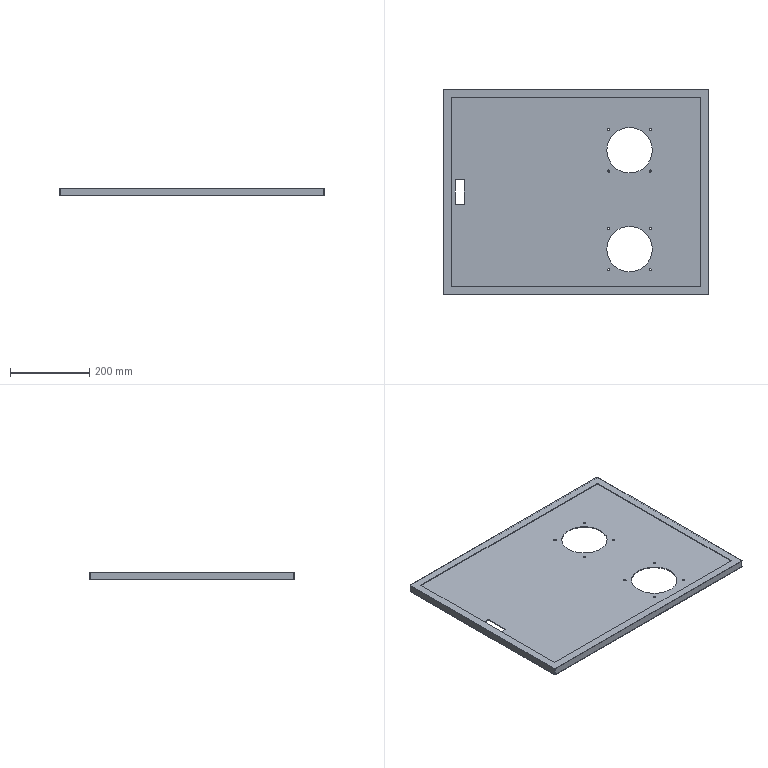Part | STEP file | 11-GYXJX-104111.111 | 1 solid | 52 faces | box 671 x 519 x 20 mm | volume 817541 mm3 | cylinder 28 | plane 20 | sphere 4 | commonest cylinder face diameters 5.5 x16 4 x8 115 x4
STEP:
#1=CARTESIAN_POINT('',(80.25,53.,2.));
#2=VERTEX_POINT('',#1);
#3=CARTESIAN_POINT('',(85.75,53.,2.));
#4=VERTEX_POINT('',#3);
#5=CARTESIAN_POINT('',(83.,53.,2.));
#6=DIRECTION('',(0.,0.,1.));
#7=DIRECTION('',(1.,0.,0.));
#8=AXIS2_PLACEMENT_3D('',#5,#6,#7);
#9=CIRCLE('',#8,2.75);
#10=EDGE_CURVE('',#2,#4,#9,.T.);
#11=ORIENTED_EDGE('',*,*,#10,.T.);
#12=CARTESIAN_POINT('',(85.75,53.,0.));
#13=VERTEX_POINT('',#12);
#14=CARTESIAN_POINT('',(85.75,53.,10.));
#15=DIRECTION('',(0.,0.,-1.));
#16=VECTOR('',#15,1000.);
#17=LINE('',#14,#16);
#18=EDGE_CURVE('',#4,#13,#17,.T.);
#19=ORIENTED_EDGE('',*,*,#18,.T.);
#20=CARTESIAN_POINT('',(80.25,53.,0.));
#21=VERTEX_POINT('',#20);
#22=CARTESIAN_POINT('',(83.,53.,0.));
#23=DIRECTION('',(0.,0.,-1.));
#24=DIRECTION('',(-1.,0.,0.));
#25=AXIS2_PLACEMENT_3D('',#22,#23,#24);
#26=CIRCLE('',#25,2.75);
#27=EDGE_CURVE('',#13,#21,#26,.T.);
#28=ORIENTED_EDGE('',*,*,#27,.T.);
#29=CARTESIAN_POINT('',(80.25,53.,10.));
#30=DIRECTION('',(0.,0.,-1.));
#31=VECTOR('',#30,1000.);
#32=LINE('',#29,#31);
#33=EDGE_CURVE('',#2,#21,#32,.T.);
#34=ORIENTED_EDGE('',*,*,#33,.F.);
#35=EDGE_LOOP('',(#11,#19,#28,#34));
#36=FACE_OUTER_BOUND('',#35,.T.);
#37=CARTESIAN_POINT('',(83.,53.,10.));
#38=DIRECTION('',(0.,0.,-1.));
#39=DIRECTION('',(-1.,0.,0.));
#40=AXIS2_PLACEMENT_3D('',#37,#38,#39);
#41=CYLINDRICAL_SURFACE('',#40,2.75);
#42=ADVANCED_FACE('',(#36),#41,.F.);
#43=CARTESIAN_POINT('',(185.25,-92.,2.));
#44=VERTEX_POINT('',#43);
#45=CARTESIAN_POINT('',(190.75,-92.,2.));
#46=VERTEX_POINT('',#45);
#47=CARTESIAN_POINT('',(188.,-92.,2.));
#48=DIRECTION('',(0.,0.,1.));
#49=DIRECTION('',(1.,0.,0.));
#50=AXIS2_PLACEMENT_3D('',#47,#48,#49);
#51=CIRCLE('',#50,2.75);
#52=EDGE_CURVE('',#44,#46,#51,.T.);
#53=ORIENTED_EDGE('',*,*,#52,.T.);
#54=CARTESIAN_POINT('',(190.75,-92.,0.));
#55=VERTEX_POINT('',#54);
#56=CARTESIAN_POINT('',(190.75,-92.,10.));
#57=DIRECTION('',(0.,0.,-1.));
#58=VECTOR('',#57,1000.);
#59=LINE('',#56,#58);
#60=EDGE_CURVE('',#46,#55,#59,.T.);
#61=ORIENTED_EDGE('',*,*,#60,.T.);
#62=CARTESIAN_POINT('',(185.25,-92.,0.));
#63=VERTEX_POINT('',#62);
#64=CARTESIAN_POINT('',(188.,-92.,0.));
#65=DIRECTION('',(0.,0.,-1.));
#66=DIRECTION('',(-1.,0.,0.));
#67=AXIS2_PLACEMENT_3D('',#64,#65,#66);
#68=CIRCLE('',#67,2.75);
#69=EDGE_CURVE('',#55,#63,#68,.T.);
#70=ORIENTED_EDGE('',*,*,#69,.T.);
#71=CARTESIAN_POINT('',(185.25,-92.,10.));
#72=DIRECTION('',(0.,0.,-1.));
#73=VECTOR('',#72,1000.);
#74=LINE('',#71,#73);
#75=EDGE_CURVE('',#44,#63,#74,.T.);
#76=ORIENTED_EDGE('',*,*,#75,.F.);
#77=EDGE_LOOP('',(#53,#61,#70,#76));
#78=FACE_OUTER_BOUND('',#77,.T.);
#79=CARTESIAN_POINT('',(188.,-92.,10.));
#80=DIRECTION('',(0.,0.,-1.));
#81=DIRECTION('',(-1.,0.,0.));
#82=AXIS2_PLACEMENT_3D('',#79,#80,#81);
#83=CYLINDRICAL_SURFACE('',#82,2.75);
#84=ADVANCED_FACE('',(#78),#83,.F.);
#85=CARTESIAN_POINT('',(80.25,-92.,2.));
#86=VERTEX_POINT('',#85);
#87=CARTESIAN_POINT('',(85.75,-92.,2.));
#88=VERTEX_POINT('',#87);
#89=CARTESIAN_POINT('',(83.,-92.,2.));
#90=DIRECTION('',(0.,0.,1.));
#91=DIRECTION('',(1.,0.,0.));
#92=AXIS2_PLACEMENT_3D('',#89,#90,#91);
#93=CIRCLE('',#92,2.75);
#94=EDGE_CURVE('',#86,#88,#93,.T.);
#95=ORIENTED_EDGE('',*,*,#94,.T.);
#96=CARTESIAN_POINT('',(85.75,-92.,0.));
#97=VERTEX_POINT('',#96);
#98=CARTESIAN_POINT('',(85.75,-92.,10.));
#99=DIRECTION('',(0.,0.,-1.));
#100=VECTOR('',#99,1000.);
#101=LINE('',#98,#100);
#102=EDGE_CURVE('',#88,#97,#101,.T.);
#103=ORIENTED_EDGE('',*,*,#102,.T.);
#104=CARTESIAN_POINT('',(80.25,-92.,0.));
#105=VERTEX_POINT('',#104);
#106=CARTESIAN_POINT('',(83.,-92.,0.));
#107=DIRECTION('',(0.,0.,-1.));
#108=DIRECTION('',(-1.,0.,0.));
#109=AXIS2_PLACEMENT_3D('',#106,#107,#108);
#110=CIRCLE('',#109,2.75);
#111=EDGE_CURVE('',#97,#105,#110,.T.);
#112=ORIENTED_EDGE('',*,*,#111,.T.);
#113=CARTESIAN_POINT('',(80.25,-92.,10.));
#114=DIRECTION('',(0.,0.,-1.));
#115=VECTOR('',#114,1000.);
#116=LINE('',#113,#115);
#117=EDGE_CURVE('',#86,#105,#116,.T.);
#118=ORIENTED_EDGE('',*,*,#117,.F.);
#119=EDGE_LOOP('',(#95,#103,#112,#118));
#120=FACE_OUTER_BOUND('',#119,.T.);
#121=CARTESIAN_POINT('',(83.,-92.,10.));
#122=DIRECTION('',(0.,0.,-1.));
#123=DIRECTION('',(-1.,0.,0.));
#124=AXIS2_PLACEMENT_3D('',#121,#122,#123);
#125=CYLINDRICAL_SURFACE('',#124,2.75);
#126=ADVANCED_FACE('',(#120),#125,.F.);
#127=CARTESIAN_POINT('',(185.25,-197.,2.));
#128=VERTEX_POINT('',#127);
#129=CARTESIAN_POINT('',(190.75,-197.,2.));
#130=VERTEX_POINT('',#129);
#131=CARTESIAN_POINT('',(188.,-197.,2.));
#132=DIRECTION('',(0.,0.,1.));
#133=DIRECTION('',(1.,0.,0.));
#134=AXIS2_PLACEMENT_3D('',#131,#132,#133);
#135=CIRCLE('',#134,2.75);
#136=EDGE_CURVE('',#128,#130,#135,.T.);
#137=ORIENTED_EDGE('',*,*,#136,.T.);
#138=CARTESIAN_POINT('',(190.75,-197.,0.));
#139=VERTEX_POINT('',#138);
#140=CARTESIAN_POINT('',(190.75,-197.,10.));
#141=DIRECTION('',(0.,0.,-1.));
#142=VECTOR('',#141,1000.);
#143=LINE('',#140,#142);
#144=EDGE_CURVE('',#130,#139,#143,.T.);
#145=ORIENTED_EDGE('',*,*,#144,.T.);
#146=CARTESIAN_POINT('',(185.25,-197.,0.));
#147=VERTEX_POINT('',#146);
#148=CARTESIAN_POINT('',(188.,-197.,0.));
#149=DIRECTION('',(0.,0.,-1.));
#150=DIRECTION('',(-1.,0.,0.));
#151=AXIS2_PLACEMENT_3D('',#148,#149,#150);
#152=CIRCLE('',#151,2.75);
#153=EDGE_CURVE('',#139,#147,#152,.T.);
#154=ORIENTED_EDGE('',*,*,#153,.T.);
#155=CARTESIAN_POINT('',(185.25,-197.,10.));
#156=DIRECTION('',(0.,0.,-1.));
#157=VECTOR('',#156,1000.);
#158=LINE('',#155,#157);
#159=EDGE_CURVE('',#128,#147,#158,.T.);
#160=ORIENTED_EDGE('',*,*,#159,.F.);
#161=EDGE_LOOP('',(#137,#145,#154,#160));
#162=FACE_OUTER_BOUND('',#161,.T.);
#163=CARTESIAN_POINT('',(188.,-197.,10.));
#164=DIRECTION('',(0.,0.,-1.));
#165=DIRECTION('',(-1.,0.,0.));
#166=AXIS2_PLACEMENT_3D('',#163,#164,#165);
#167=CYLINDRICAL_SURFACE('',#166,2.75);
#168=ADVANCED_FACE('',(#162),#167,.F.);
#169=CARTESIAN_POINT('',(80.25,-197.,2.));
#170=VERTEX_POINT('',#169);
#171=CARTESIAN_POINT('',(85.75,-197.,2.));
#172=VERTEX_POINT('',#171);
#173=CARTESIAN_POINT('',(83.,-197.,2.));
#174=DIRECTION('',(0.,0.,1.));
#175=DIRECTION('',(1.,0.,0.));
#176=AXIS2_PLACEMENT_3D('',#173,#174,#175);
#177=CIRCLE('',#176,2.75);
#178=EDGE_CURVE('',#170,#172,#177,.T.);
#179=ORIENTED_EDGE('',*,*,#178,.T.);
#180=CARTESIAN_POINT('',(85.75,-197.,0.));
#181=VERTEX_POINT('',#180);
#182=CARTESIAN_POINT('',(85.75,-197.,10.));
#183=DIRECTION('',(0.,0.,-1.));
#184=VECTOR('',#183,1000.);
#185=LINE('',#182,#184);
#186=EDGE_CURVE('',#172,#181,#185,.T.);
#187=ORIENTED_EDGE('',*,*,#186,.T.);
#188=CARTESIAN_POINT('',(80.25,-197.,0.));
#189=VERTEX_POINT('',#188);
#190=CARTESIAN_POINT('',(83.,-197.,0.));
#191=DIRECTION('',(0.,0.,-1.));
#192=DIRECTION('',(-1.,0.,0.));
#193=AXIS2_PLACEMENT_3D('',#190,#191,#192);
#194=CIRCLE('',#193,2.75);
#195=EDGE_CURVE('',#181,#189,#194,.T.);
#196=ORIENTED_EDGE('',*,*,#195,.T.);
#197=CARTESIAN_POINT('',(80.25,-197.,10.));
#198=DIRECTION('',(0.,0.,-1.));
#199=VECTOR('',#198,1000.);
#200=LINE('',#197,#199);
#201=EDGE_CURVE('',#170,#189,#200,.T.);
#202=ORIENTED_EDGE('',*,*,#201,.F.);
#203=EDGE_LOOP('',(#179,#187,#196,#202));
#204=FACE_OUTER_BOUND('',#203,.T.);
#205=CARTESIAN_POINT('',(83.,-197.,10.));
#206=DIRECTION('',(0.,0.,-1.));
#207=DIRECTION('',(-1.,0.,0.));
#208=AXIS2_PLACEMENT_3D('',#205,#206,#207);
#209=CYLINDRICAL_SURFACE('',#208,2.75);
#210=ADVANCED_FACE('',(#204),#209,.F.);
#211=CARTESIAN_POINT('',(78.,-144.5,2.));
#212=VERTEX_POINT('',#211);
#213=CARTESIAN_POINT('',(193.,-144.5,2.));
#214=VERTEX_POINT('',#213);
#215=CARTESIAN_POINT('',(135.5,-144.5,2.));
#216=DIRECTION('',(0.,0.,1.));
#217=DIRECTION('',(1.,0.,0.));
#218=AXIS2_PLACEMENT_3D('',#215,#216,#217);
#219=CIRCLE('',#218,57.5);
#220=EDGE_CURVE('',#212,#214,#219,.T.);
#221=ORIENTED_EDGE('',*,*,#220,.T.);
#222=CARTESIAN_POINT('',(193.,-144.5,0.));
#223=VERTEX_POINT('',#222);
#224=CARTESIAN_POINT('',(193.,-144.5,10.));
#225=DIRECTION('',(0.,0.,-1.));
#226=VECTOR('',#225,1000.);
#227=LINE('',#224,#226);
#228=EDGE_CURVE('',#214,#223,#227,.T.);
#229=ORIENTED_EDGE('',*,*,#228,.T.);
#230=CARTESIAN_POINT('',(78.,-144.5,0.));
#231=VERTEX_POINT('',#230);
#232=CARTESIAN_POINT('',(135.5,-144.5,0.));
#233=DIRECTION('',(0.,0.,-1.));
#234=DIRECTION('',(-1.,0.,0.));
#235=AXIS2_PLACEMENT_3D('',#232,#233,#234);
#236=CIRCLE('',#235,57.5);
#237=EDGE_CURVE('',#223,#231,#236,.T.);
#238=ORIENTED_EDGE('',*,*,#237,.T.);
#239=CARTESIAN_POINT('',(78.,-144.5,10.));
#240=DIRECTION('',(0.,0.,-1.));
#241=VECTOR('',#240,1000.);
#242=LINE('',#239,#241);
#243=EDGE_CURVE('',#212,#231,#242,.T.);
#244=ORIENTED_EDGE('',*,*,#243,.F.);
#245=EDGE_LOOP('',(#221,#229,#238,#244));
#246=FACE_OUTER_BOUND('',#245,.T.);
#247=CARTESIAN_POINT('',(135.5,-144.5,10.));
#248=DIRECTION('',(0.,0.,-1.));
#249=DIRECTION('',(-1.,0.,0.));
#250=AXIS2_PLACEMENT_3D('',#247,#248,#249);
#251=CYLINDRICAL_SURFACE('',#250,57.5);
#252=ADVANCED_FACE('',(#246),#251,.F.);
#253=CARTESIAN_POINT('',(185.25,158.,2.));
#254=VERTEX_POINT('',#253);
#255=CARTESIAN_POINT('',(190.75,158.,2.));
#256=VERTEX_POINT('',#255);
#257=CARTESIAN_POINT('',(188.,158.,2.));
#258=DIRECTION('',(0.,0.,1.));
#259=DIRECTION('',(1.,0.,0.));
#260=AXIS2_PLACEMENT_3D('',#257,#258,#259);
#261=CIRCLE('',#260,2.75);
#262=EDGE_CURVE('',#254,#256,#261,.T.);
#263=ORIENTED_EDGE('',*,*,#262,.T.);
#264=CARTESIAN_POINT('',(190.75,158.,0.));
#265=VERTEX_POINT('',#264);
#266=CARTESIAN_POINT('',(190.75,158.,10.));
#267=DIRECTION('',(0.,0.,-1.));
#268=VECTOR('',#267,1000.);
#269=LINE('',#266,#268);
#270=EDGE_CURVE('',#256,#265,#269,.T.);
#271=ORIENTED_EDGE('',*,*,#270,.T.);
#272=CARTESIAN_POINT('',(185.25,158.,0.));
#273=VERTEX_POINT('',#272);
#274=CARTESIAN_POINT('',(188.,158.,0.));
#275=DIRECTION('',(0.,0.,-1.));
#276=DIRECTION('',(-1.,0.,0.));
#277=AXIS2_PLACEMENT_3D('',#274,#275,#276);
#278=CIRCLE('',#277,2.75);
#279=EDGE_CURVE('',#265,#273,#278,.T.);
#280=ORIENTED_EDGE('',*,*,#279,.T.);
#281=CARTESIAN_POINT('',(185.25,158.,10.));
#282=DIRECTION('',(0.,0.,-1.));
#283=VECTOR('',#282,1000.);
#284=LINE('',#281,#283);
#285=EDGE_CURVE('',#254,#273,#284,.T.);
#286=ORIENTED_EDGE('',*,*,#285,.F.);
#287=EDGE_LOOP('',(#263,#271,#280,#286));
#288=FACE_OUTER_BOUND('',#287,.T.);
#289=CARTESIAN_POINT('',(188.,158.,10.));
#290=DIRECTION('',(0.,0.,-1.));
#291=DIRECTION('',(-1.,0.,0.));
#292=AXIS2_PLACEMENT_3D('',#289,#290,#291);
#293=CYLINDRICAL_SURFACE('',#292,2.75);
#294=ADVANCED_FACE('',(#288),#293,.F.);
#295=CARTESIAN_POINT('',(80.25,158.,2.));
#296=VERTEX_POINT('',#295);
#297=CARTESIAN_POINT('',(85.75,158.,2.));
#298=VERTEX_POINT('',#297);
#299=CARTESIAN_POINT('',(83.,158.,2.));
#300=DIRECTION('',(0.,0.,1.));
#301=DIRECTION('',(1.,0.,0.));
#302=AXIS2_PLACEMENT_3D('',#299,#300,#301);
#303=CIRCLE('',#302,2.75);
#304=EDGE_CURVE('',#296,#298,#303,.T.);
#305=ORIENTED_EDGE('',*,*,#304,.T.);
#306=CARTESIAN_POINT('',(85.75,158.,0.));
#307=VERTEX_POINT('',#306);
#308=CARTESIAN_POINT('',(85.75,158.,10.));
#309=DIRECTION('',(0.,0.,-1.));
#310=VECTOR('',#309,1000.);
#311=LINE('',#308,#310);
#312=EDGE_CURVE('',#298,#307,#311,.T.);
#313=ORIENTED_EDGE('',*,*,#312,.T.);
#314=CARTESIAN_POINT('',(80.25,158.,0.));
#315=VERTEX_POINT('',#314);
#316=CARTESIAN_POINT('',(83.,158.,0.));
#317=DIRECTION('',(0.,0.,-1.));
#318=DIRECTION('',(-1.,0.,0.));
#319=AXIS2_PLACEMENT_3D('',#316,#317,#318);
#320=CIRCLE('',#319,2.75);
#321=EDGE_CURVE('',#307,#315,#320,.T.);
#322=ORIENTED_EDGE('',*,*,#321,.T.);
#323=CARTESIAN_POINT('',(80.25,158.,10.));
#324=DIRECTION('',(0.,0.,-1.));
#325=VECTOR('',#324,1000.);
#326=LINE('',#323,#325);
#327=EDGE_CURVE('',#296,#315,#326,.T.);
#328=ORIENTED_EDGE('',*,*,#327,.F.);
#329=EDGE_LOOP('',(#305,#313,#322,#328));
#330=FACE_OUTER_BOUND('',#329,.T.);
#331=CARTESIAN_POINT('',(83.,158.,10.));
#332=DIRECTION('',(0.,0.,-1.));
#333=DIRECTION('',(-1.,0.,0.));
#334=AXIS2_PLACEMENT_3D('',#331,#332,#333);
#335=CYLINDRICAL_SURFACE('',#334,2.75);
#336=ADVANCED_FACE('',(#330),#335,.F.);
#337=CARTESIAN_POINT('',(185.25,53.,2.));
#338=VERTEX_POINT('',#337);
#339=CARTESIAN_POINT('',(190.75,53.,2.));
#340=VERTEX_POINT('',#339);
#341=CARTESIAN_POINT('',(188.,53.,2.));
#342=DIRECTION('',(0.,0.,1.));
#343=DIRECTION('',(1.,0.,0.));
#344=AXIS2_PLACEMENT_3D('',#341,#342,#343);
#345=CIRCLE('',#344,2.75);
#346=EDGE_CURVE('',#338,#340,#345,.T.);
#347=ORIENTED_EDGE('',*,*,#346,.T.);
#348=CARTESIAN_POINT('',(190.75,53.,0.));
#349=VERTEX_POINT('',#348);
#350=CARTESIAN_POINT('',(190.75,53.,10.));
#351=DIRECTION('',(0.,0.,-1.));
#352=VECTOR('',#351,1000.);
#353=LINE('',#350,#352);
#354=EDGE_CURVE('',#340,#349,#353,.T.);
#355=ORIENTED_EDGE('',*,*,#354,.T.);
#356=CARTESIAN_POINT('',(185.25,53.,0.));
#357=VERTEX_POINT('',#356);
#358=CARTESIAN_POINT('',(188.,53.,0.));
#359=DIRECTION('',(0.,0.,-1.));
#360=DIRECTION('',(-1.,0.,0.));
#361=AXIS2_PLACEMENT_3D('',#358,#359,#360);
#362=CIRCLE('',#361,2.75);
#363=EDGE_CURVE('',#349,#357,#362,.T.);
#364=ORIENTED_EDGE('',*,*,#363,.T.);
#365=CARTESIAN_POINT('',(185.25,53.,10.));
#366=DIRECTION('',(0.,0.,-1.));
#367=VECTOR('',#366,1000.);
#368=LINE('',#365,#367);
#369=EDGE_CURVE('',#338,#357,#368,.T.);
#370=ORIENTED_EDGE('',*,*,#369,.F.);
#371=EDGE_LOOP('',(#347,#355,#364,#370));
#372=FACE_OUTER_BOUND('',#371,.T.);
#373=CARTESIAN_POINT('',(188.,53.,10.));
#374=DIRECTION('',(0.,0.,-1.));
#375=DIRECTION('',(-1.,0.,0.));
#376=AXIS2_PLACEMENT_3D('',#373,#374,#375);
#377=CYLINDRICAL_SURFACE('',#376,2.75);
#378=ADVANCED_FACE('',(#372),#377,.F.);
#379=CARTESIAN_POINT('',(78.,105.5,2.));
#380=VERTEX_POINT('',#379);
#381=CARTESIAN_POINT('',(193.,105.5,2.));
#382=VERTEX_POINT('',#381);
#383=CARTESIAN_POINT('',(135.5,105.5,2.));
#384=DIRECTION('',(0.,0.,1.));
#385=DIRECTION('',(1.,0.,0.));
#386=AXIS2_PLACEMENT_3D('',#383,#384,#385);
#387=CIRCLE('',#386,57.5);
#388=EDGE_CURVE('',#380,#382,#387,.T.);
#389=ORIENTED_EDGE('',*,*,#388,.T.);
#390=CARTESIAN_POINT('',(193.,105.5,0.));
#391=VERTEX_POINT('',#390);
#392=CARTESIAN_POINT('',(193.,105.5,10.));
#393=DIRECTION('',(0.,0.,-1.));
#394=VECTOR('',#393,1000.);
#395=LINE('',#392,#394);
#396=EDGE_CURVE('',#382,#391,#395,.T.);
#397=ORIENTED_EDGE('',*,*,#396,.T.);
#398=CARTESIAN_POINT('',(78.,105.5,0.));
#399=VERTEX_POINT('',#398);
#400=CARTESIAN_POINT('',(135.5,105.5,0.));
#401=DIRECTION('',(0.,0.,-1.));
#402=DIRECTION('',(-1.,0.,0.));
#403=AXIS2_PLACEMENT_3D('',#400,#401,#402);
#404=CIRCLE('',#403,57.5);
#405=EDGE_CURVE('',#391,#399,#404,.T.);
#406=ORIENTED_EDGE('',*,*,#405,.T.);
#407=CARTESIAN_POINT('',(78.,105.5,10.));
#408=DIRECTION('',(0.,0.,-1.));
#409=VECTOR('',#408,1000.);
#410=LINE('',#407,#409);
#411=EDGE_CURVE('',#380,#399,#410,.T.);
#412=ORIENTED_EDGE('',*,*,#411,.F.);
#413=EDGE_LOOP('',(#389,#397,#406,#412));
#414=FACE_OUTER_BOUND('',#413,.T.);
#415=CARTESIAN_POINT('',(135.5,105.5,10.));
#416=DIRECTION('',(0.,0.,-1.));
#417=DIRECTION('',(-1.,0.,0.));
#418=AXIS2_PLACEMENT_3D('',#415,#416,#417);
#419=CYLINDRICAL_SURFACE('',#418,57.5);
#420=ADVANCED_FACE('',(#414),#419,.F.);
#421=CARTESIAN_POINT('',(335.5,-257.5,2.));
#422=VERTEX_POINT('',#421);
#423=CARTESIAN_POINT('',(335.5,257.5,2.));
#424=VERTEX_POINT('',#423);
#425=CARTESIAN_POINT('',(335.5,259.5,2.));
#426=DIRECTION('',(0.,1.,0.));
#427=VECTOR('',#426,1000.);
#428=LINE('',#425,#427);
#429=EDGE_CURVE('',#422,#424,#428,.T.);
#430=ORIENTED_EDGE('',*,*,#429,.T.);
#431=CARTESIAN_POINT('',(335.5,257.5,20.));
#432=VERTEX_POINT('',#431);
#433=CARTESIAN_POINT('',(335.5,257.5,20.));
#434=DIRECTION('',(0.,0.,1.));
#435=VECTOR('',#434,1000.);
#436=LINE('',#433,#435);
#437=EDGE_CURVE('',#424,#432,#436,.T.);
#438=ORIENTED_EDGE('',*,*,#437,.T.);
#439=CARTESIAN_POINT('',(335.5,-257.5,20.));
#440=VERTEX_POINT('',#439);
#441=CARTESIAN_POINT('',(335.5,259.5,20.));
#442=DIRECTION('',(0.,1.,0.));
#443=VECTOR('',#442,1000.);
#444=LINE('',#441,#443);
#445=EDGE_CURVE('',#440,#432,#444,.T.);
#446=ORIENTED_EDGE('',*,*,#445,.F.);
#447=CARTESIAN_POINT('',(335.5,-257.5,20.));
#448=DIRECTION('',(0.,0.,-1.));
#449=VECTOR('',#448,1000.);
#450=LINE('',#447,#449);
#451=EDGE_CURVE('',#440,#422,#450,.T.);
#452=ORIENTED_EDGE('',*,*,#451,.T.);
#453=EDGE_LOOP('',(#430,#438,#446,#452));
#454=FACE_OUTER_BOUND('',#453,.T.);
#455=CARTESIAN_POINT('',(335.5,259.5,20.));
#456=DIRECTION('',(-1.,0.,0.));
#457=DIRECTION('',(0.,-1.,0.));
#458=AXIS2_PLACEMENT_3D('',#455,#456,#457);
#459=PLANE('',#458);
#460=ADVANCED_FACE('',(#454),#459,.F.);
#461=CARTESIAN_POINT('',(333.5,259.5,2.));
#462=VERTEX_POINT('',#461);
#463=CARTESIAN_POINT('',(-333.5,259.5,2.));
#464=VERTEX_POINT('',#463);
#465=CARTESIAN_POINT('',(-335.5,259.5,2.));
#466=DIRECTION('',(-1.,0.,0.));
#467=VECTOR('',#466,1000.);
#468=LINE('',#465,#467);
#469=EDGE_CURVE('',#462,#464,#468,.T.);
#470=ORIENTED_EDGE('',*,*,#469,.T.);
#471=CARTESIAN_POINT('',(-333.5,259.5,20.));
#472=VERTEX_POINT('',#471);
#473=CARTESIAN_POINT('',(-333.5,259.5,20.));
#474=DIRECTION('',(0.,0.,1.));
#475=VECTOR('',#474,1000.);
#476=LINE('',#473,#475);
#477=EDGE_CURVE('',#464,#472,#476,.T.);
#478=ORIENTED_EDGE('',*,*,#477,.T.);
#479=CARTESIAN_POINT('',(333.5,259.5,20.));
#480=VERTEX_POINT('',#479);
#481=CARTESIAN_POINT('',(-335.5,259.5,20.));
#482=DIRECTION('',(-1.,0.,0.));
#483=VECTOR('',#482,1000.);
#484=LINE('',#481,#483);
#485=EDGE_CURVE('',#480,#472,#484,.T.);
#486=ORIENTED_EDGE('',*,*,#485,.F.);
#487=CARTESIAN_POINT('',(333.5,259.5,20.));
#488=DIRECTION('',(0.,0.,-1.));
#489=VECTOR('',#488,1000.);
#490=LINE('',#487,#489);
#491=EDGE_CURVE('',#480,#462,#490,.T.);
#492=ORIENTED_EDGE('',*,*,#491,.T.);
#493=EDGE_LOOP('',(#470,#478,#486,#492));
#494=FACE_OUTER_BOUND('',#493,.T.);
#495=CARTESIAN_POINT('',(-335.5,259.5,20.));
#496=DIRECTION('',(0.,-1.,0.));
#497=DIRECTION('',(0.,0.,-1.));
#498=AXIS2_PLACEMENT_3D('',#495,#496,#497);
#499=PLANE('',#498);
#500=ADVANCED_FACE('',(#494),#499,.F.);
#501=CARTESIAN_POINT('',(-335.5,257.5,20.));
#502=VERTEX_POINT('',#501);
#503=CARTESIAN_POINT('',(-335.5,-257.5,20.));
#504=VERTEX_POINT('',#503);
#505=CARTESIAN_POINT('',(-335.5,259.5,20.));
#506=DIRECTION('',(0.,-1.,0.));
#507=VECTOR('',#506,1000.);
#508=LINE('',#505,#507);
#509=EDGE_CURVE('',#502,#504,#508,.T.);
#510=ORIENTED_EDGE('',*,*,#509,.F.);
#511=CARTESIAN_POINT('',(-335.5,257.5,2.));
#512=VERTEX_POINT('',#511);
#513=CARTESIAN_POINT('',(-335.5,257.5,20.));
#514=DIRECTION('',(0.,0.,-1.));
#515=VECTOR('',#514,1000.);
#516=LINE('',#513,#515);
#517=EDGE_CURVE('',#502,#512,#516,.T.);
#518=ORIENTED_EDGE('',*,*,#517,.T.);
#519=CARTESIAN_POINT('',(-335.5,-257.5,2.));
#520=VERTEX_POINT('',#519);
#521=CARTESIAN_POINT('',(-335.5,259.5,2.));
#522=DIRECTION('',(0.,-1.,0.));
#523=VECTOR('',#522,1000.);
#524=LINE('',#521,#523);
#525=EDGE_CURVE('',#512,#520,#524,.T.);
#526=ORIENTED_EDGE('',*,*,#525,.T.);
#527=CARTESIAN_POINT('',(-335.5,-257.5,20.));
#528=DIRECTION('',(0.,0.,1.));
#529=VECTOR('',#528,1000.);
#530=LINE('',#527,#529);
#531=EDGE_CURVE('',#520,#504,#530,.T.);
#532=ORIENTED_EDGE('',*,*,#531,.T.);
#533=EDGE_LOOP('',(#510,#518,#526,#532));
#534=FACE_OUTER_BOUND('',#533,.T.);
#535=CARTESIAN_POINT('',(-335.5,259.5,20.));
#536=DIRECTION('',(1.,0.,0.));
#537=DIRECTION('',(0.,0.,-1.));
#538=AXIS2_PLACEMENT_3D('',#535,#536,#537);
#539=PLANE('',#538);
#540=ADVANCED_FACE('',(#534),#539,.F.);
#541=CARTESIAN_POINT('',(-333.5,-259.5,2.));
#542=VERTEX_POINT('',#541);
#543=CARTESIAN_POINT('',(333.5,-259.5,2.));
#544=VERTEX_POINT('',#543);
#545=CARTESIAN_POINT('',(-335.5,-259.5,2.));
#546=DIRECTION('',(1.,0.,0.));
#547=VECTOR('',#546,1000.);
#548=LINE('',#545,#547);
#549=EDGE_CURVE('',#542,#544,#548,.T.);
#550=ORIENTED_EDGE('',*,*,#549,.T.);
#551=CARTESIAN_POINT('',(333.5,-259.5,20.));
#552=VERTEX_POINT('',#551);
#553=CARTESIAN_POINT('',(333.5,-259.5,20.));
#554=DIRECTION('',(0.,0.,1.));
#555=VECTOR('',#554,1000.);
#556=LINE('',#553,#555);
#557=EDGE_CURVE('',#544,#552,#556,.T.);
#558=ORIENTED_EDGE('',*,*,#557,.T.);
#559=CARTESIAN_POINT('',(-333.5,-259.5,20.));
#560=VERTEX_POINT('',#559);
#561=CARTESIAN_POINT('',(-335.5,-259.5,20.));
#562=DIRECTION('',(1.,0.,0.));
#563=VECTOR('',#562,1000.);
#564=LINE('',#561,#563);
#565=EDGE_CURVE('',#560,#552,#564,.T.);
#566=ORIENTED_EDGE('',*,*,#565,.F.);
#567=CARTESIAN_POINT('',(-333.5,-259.5,20.));
#568=DIRECTION('',(0.,0.,-1.));
#569=VECTOR('',#568,1000.);
#570=LINE('',#567,#569);
#571=EDGE_CURVE('',#560,#542,#570,.T.);
#572=ORIENTED_EDGE('',*,*,#571,.T.);
#573=EDGE_LOOP('',(#550,#558,#566,#572));
#574=FACE_OUTER_BOUND('',#573,.T.);
#575=CARTESIAN_POINT('',(-335.5,-259.5,20.));
#576=DIRECTION('',(0.,1.,0.));
#577=DIRECTION('',(0.,0.,1.));
#578=AXIS2_PLACEMENT_3D('',#575,#576,#577);
#579=PLANE('',#578);
#580=ADVANCED_FACE('',(#574),#579,.F.);
#581=ORIENTED_EDGE('',*,*,#485,.T.);
#582=CARTESIAN_POINT('',(-333.5,257.5,20.));
#583=DIRECTION('',(0.,0.,1.));
#584=DIRECTION('',(1.,0.,0.));
#585=AXIS2_PLACEMENT_3D('',#582,#583,#584);
#586=CIRCLE('',#585,2.);
#587=EDGE_CURVE('',#472,#502,#586,.T.);
#588=ORIENTED_EDGE('',*,*,#587,.T.);
#589=ORIENTED_EDGE('',*,*,#509,.T.);
#590=CARTESIAN_POINT('',(-333.5,-257.5,20.));
#591=DIRECTION('',(0.,0.,1.));
#592=DIRECTION('',(1.,0.,0.));
#593=AXIS2_PLACEMENT_3D('',#590,#591,#592);
#594=CIRCLE('',#593,2.);
#595=EDGE_CURVE('',#504,#560,#594,.T.);
#596=ORIENTED_EDGE('',*,*,#595,.T.);
#597=ORIENTED_EDGE('',*,*,#565,.T.);
#598=CARTESIAN_POINT('',(333.5,-257.5,20.));
#599=DIRECTION('',(0.,0.,1.));
#600=DIRECTION('',(1.,0.,0.));
#601=AXIS2_PLACEMENT_3D('',#598,#599,#600);
#602=CIRCLE('',#601,2.);
#603=EDGE_CURVE('',#552,#440,#602,.T.);
#604=ORIENTED_EDGE('',*,*,#603,.T.);
#605=ORIENTED_EDGE('',*,*,#445,.T.);
#606=CARTESIAN_POINT('',(333.5,257.5,20.));
#607=DIRECTION('',(0.,0.,1.));
#608=DIRECTION('',(1.,0.,0.));
#609=AXIS2_PLACEMENT_3D('',#606,#607,#608);
#610=CIRCLE('',#609,2.);
#611=EDGE_CURVE('',#432,#480,#610,.T.);
#612=ORIENTED_EDGE('',*,*,#611,.T.);
#613=EDGE_LOOP('',(#581,#588,#589,#596,#597,#604,#605,#612));
#614=FACE_OUTER_BOUND('',#613,.T.);
#615=CARTESIAN_POINT('',(-315.5,239.5,20.));
#616=VERTEX_POINT('',#615);
#617=CARTESIAN_POINT('',(-315.5,-239.5,20.));
#618=VERTEX_POINT('',#617);
#619=CARTESIAN_POINT('',(-315.5,257.5,20.));
#620=DIRECTION('',(0.,-1.,0.));
#621=VECTOR('',#620,1000.);
#622=LINE('',#619,#621);
#623=EDGE_CURVE('',#616,#618,#622,.T.);
#624=ORIENTED_EDGE('',*,*,#623,.F.);
#625=CARTESIAN_POINT('',(315.5,239.5,20.));
#626=VERTEX_POINT('',#625);
#627=CARTESIAN_POINT('',(-333.5,239.5,20.));
#628=DIRECTION('',(-1.,0.,0.));
#629=VECTOR('',#628,1000.);
#630=LINE('',#627,#629);
#631=EDGE_CURVE('',#626,#616,#630,.T.);
#632=ORIENTED_EDGE('',*,*,#631,.F.);
#633=CARTESIAN_POINT('',(315.5,-239.5,20.));
#634=VERTEX_POINT('',#633);
#635=CARTESIAN_POINT('',(315.5,257.5,20.));
#636=DIRECTION('',(0.,1.,0.));
#637=VECTOR('',#636,1000.);
#638=LINE('',#635,#637);
#639=EDGE_CURVE('',#634,#626,#638,.T.);
#640=ORIENTED_EDGE('',*,*,#639,.F.);
#641=CARTESIAN_POINT('',(-333.5,-239.5,20.));
#642=DIRECTION('',(1.,0.,0.));
#643=VECTOR('',#642,1000.);
#644=LINE('',#641,#643);
#645=EDGE_CURVE('',#618,#634,#644,.T.);
#646=ORIENTED_EDGE('',*,*,#645,.F.);
#647=EDGE_LOOP('',(#624,#632,#640,#646));
#648=FACE_BOUND('',#647,.T.);
#649=CARTESIAN_POINT('',(0.,0.,20.));
#650=DIRECTION('',(0.,0.,1.));
#651=DIRECTION('',(1.,0.,0.));
#652=AXIS2_PLACEMENT_3D('',#649,#650,#651);
#653=PLANE('',#652);
#654=ADVANCED_FACE('',(#614,#648),#653,.T.);
#655=CARTESIAN_POINT('',(83.,53.,0.));
#656=DIRECTION('',(0.,0.,-1.));
#657=DIRECTION('',(-1.,0.,0.));
#658=AXIS2_PLACEMENT_3D('',#655,#656,#657);
#659=CIRCLE('',#658,2.75);
#660=EDGE_CURVE('',#21,#13,#659,.T.);
#661=ORIENTED_EDGE('',*,*,#660,.F.);
#662=ORIENTED_EDGE('',*,*,#27,.F.);
#663=EDGE_LOOP('',(#661,#662));
#664=FACE_BOUND('',#663,.T.);
#665=CARTESIAN_POINT('',(188.,-92.,0.));
#666=DIRECTION('',(0.,0.,-1.));
#667=DIRECTION('',(-1.,0.,0.));
#668=AXIS2_PLACEMENT_3D('',#665,#666,#667);
#669=CIRCLE('',#668,2.75);
#670=EDGE_CURVE('',#63,#55,#669,.T.);
#671=ORIENTED_EDGE('',*,*,#670,.F.);
#672=ORIENTED_EDGE('',*,*,#69,.F.);
#673=EDGE_LOOP('',(#671,#672));
#674=FACE_BOUND('',#673,.T.);
#675=CARTESIAN_POINT('',(83.,-92.,0.));
#676=DIRECTION('',(0.,0.,-1.));
#677=DIRECTION('',(-1.,0.,0.));
#678=AXIS2_PLACEMENT_3D('',#675,#676,#677);
#679=CIRCLE('',#678,2.75);
#680=EDGE_CURVE('',#105,#97,#679,.T.);
#681=ORIENTED_EDGE('',*,*,#680,.F.);
#682=ORIENTED_EDGE('',*,*,#111,.F.);
#683=EDGE_LOOP('',(#681,#682));
#684=FACE_BOUND('',#683,.T.);
#685=CARTESIAN_POINT('',(188.,-197.,0.));
#686=DIRECTION('',(0.,0.,-1.));
#687=DIRECTION('',(-1.,0.,0.));
#688=AXIS2_PLACEMENT_3D('',#685,#686,#687);
#689=CIRCLE('',#688,2.75);
#690=EDGE_CURVE('',#147,#139,#689,.T.);
#691=ORIENTED_EDGE('',*,*,#690,.F.);
#692=ORIENTED_EDGE('',*,*,#153,.F.);
#693=EDGE_LOOP('',(#691,#692));
#694=FACE_BOUND('',#693,.T.);
#695=CARTESIAN_POINT('',(83.,-197.,0.));
#696=DIRECTION('',(0.,0.,-1.));
#697=DIRECTION('',(-1.,0.,0.));
#698=AXIS2_PLACEMENT_3D('',#695,#696,#697);
#699=CIRCLE('',#698,2.75);
#700=EDGE_CURVE('',#189,#181,#699,.T.);
#701=ORIENTED_EDGE('',*,*,#700,.F.);
#702=ORIENTED_EDGE('',*,*,#195,.F.);
#703=EDGE_LOOP('',(#701,#702));
#704=FACE_BOUND('',#703,.T.);
#705=CARTESIAN_POINT('',(135.5,-144.5,0.));
#706=DIRECTION('',(0.,0.,-1.));
#707=DIRECTION('',(-1.,0.,0.));
#708=AXIS2_PLACEMENT_3D('',#705,#706,#707);
#709=CIRCLE('',#708,57.5);
#710=EDGE_CURVE('',#231,#223,#709,.T.);
#711=ORIENTED_EDGE('',*,*,#710,.F.);
#712=ORIENTED_EDGE('',*,*,#237,.F.);
#713=EDGE_LOOP('',(#711,#712));
#714=FACE_BOUND('',#713,.T.);
#715=CARTESIAN_POINT('',(188.,158.,0.));
#716=DIRECTION('',(0.,0.,-1.));
#717=DIRECTION('',(-1.,0.,0.));
#718=AXIS2_PLACEMENT_3D('',#715,#716,#717);
#719=CIRCLE('',#718,2.75);
#720=EDGE_CURVE('',#273,#265,#719,.T.);
#721=ORIENTED_EDGE('',*,*,#720,.F.);
#722=ORIENTED_EDGE('',*,*,#279,.F.);
#723=EDGE_LOOP('',(#721,#722));
#724=FACE_BOUND('',#723,.T.);
#725=CARTESIAN_POINT('',(83.,158.,0.));
#726=DIRECTION('',(0.,0.,-1.));
#727=DIRECTION('',(-1.,0.,0.));
#728=AXIS2_PLACEMENT_3D('',#725,#726,#727);
#729=CIRCLE('',#728,2.75);
#730=EDGE_CURVE('',#315,#307,#729,.T.);
#731=ORIENTED_EDGE('',*,*,#730,.F.);
#732=ORIENTED_EDGE('',*,*,#321,.F.);
#733=EDGE_LOOP('',(#731,#732));
#734=FACE_BOUND('',#733,.T.);
#735=CARTESIAN_POINT('',(188.,53.,0.));
#736=DIRECTION('',(0.,0.,-1.));
#737=DIRECTION('',(-1.,0.,0.));
#738=AXIS2_PLACEMENT_3D('',#735,#736,#737);
#739=CIRCLE('',#738,2.75);
#740=EDGE_CURVE('',#357,#349,#739,.T.);
#741=ORIENTED_EDGE('',*,*,#740,.F.);
#742=ORIENTED_EDGE('',*,*,#363,.F.);
#743=EDGE_LOOP('',(#741,#742));
#744=FACE_BOUND('',#743,.T.);
#745=CARTESIAN_POINT('',(135.5,105.5,0.));
#746=DIRECTION('',(0.,0.,-1.));
#747=DIRECTION('',(-1.,0.,0.));
#748=AXIS2_PLACEMENT_3D('',#745,#746,#747);
#749=CIRCLE('',#748,57.5);
#750=EDGE_CURVE('',#399,#391,#749,.T.);
#751=ORIENTED_EDGE('',*,*,#750,.F.);
#752=ORIENTED_EDGE('',*,*,#405,.F.);
#753=EDGE_LOOP('',(#751,#752));
#754=FACE_BOUND('',#753,.T.);
#755=CARTESIAN_POINT('',(-333.5,-257.5,0.));
#756=VERTEX_POINT('',#755);
#757=CARTESIAN_POINT('',(-333.5,257.5,0.));
#758=VERTEX_POINT('',#757);
#759=CARTESIAN_POINT('',(-333.5,0.,0.));
#760=DIRECTION('',(0.,1.,0.));
#761=VECTOR('',#760,1000.);
#762=LINE('',#759,#761);
#763=EDGE_CURVE('',#756,#758,#762,.T.);
#764=ORIENTED_EDGE('',*,*,#763,.T.);
#765=CARTESIAN_POINT('',(333.5,257.5,0.));
#766=VERTEX_POINT('',#765);
#767=CARTESIAN_POINT('',(0.,257.5,0.));
#768=DIRECTION('',(1.,0.,0.));
#769=VECTOR('',#768,1000.);
#770=LINE('',#767,#769);
#771=EDGE_CURVE('',#758,#766,#770,.T.);
#772=ORIENTED_EDGE('',*,*,#771,.T.);
#773=CARTESIAN_POINT('',(333.5,-257.5,0.));
#774=VERTEX_POINT('',#773);
#775=CARTESIAN_POINT('',(333.5,0.,0.));
#776=DIRECTION('',(0.,-1.,0.));
#777=VECTOR('',#776,1000.);
#778=LINE('',#775,#777);
#779=EDGE_CURVE('',#766,#774,#778,.T.);
#780=ORIENTED_EDGE('',*,*,#779,.T.);
#781=CARTESIAN_POINT('',(0.,-257.5,0.));
#782=DIRECTION('',(-1.,0.,0.));
#783=VECTOR('',#782,1000.);
#784=LINE('',#781,#783);
#785=EDGE_CURVE('',#774,#756,#784,.T.);
#786=ORIENTED_EDGE('',*,*,#785,.T.);
#787=EDGE_LOOP('',(#764,#772,#780,#786));
#788=FACE_OUTER_BOUND('',#787,.T.);
#789=CARTESIAN_POINT('',(-305.5,-31.,0.));
#790=VERTEX_POINT('',#789);
#791=CARTESIAN_POINT('',(-282.7,-31.,0.));
#792=VERTEX_POINT('',#791);
#793=CARTESIAN_POINT('',(-282.7,-31.,0.));
#794=DIRECTION('',(1.,0.,0.));
#795=VECTOR('',#794,1000.);
#796=LINE('',#793,#795);
#797=EDGE_CURVE('',#790,#792,#796,.T.);
#798=ORIENTED_EDGE('',*,*,#797,.T.);
#799=CARTESIAN_POINT('',(-282.7,31.,0.));
#800=VERTEX_POINT('',#799);
#801=CARTESIAN_POINT('',(-282.7,31.,0.));
#802=DIRECTION('',(0.,1.,0.));
#803=VECTOR('',#802,1000.);
#804=LINE('',#801,#803);
#805=EDGE_CURVE('',#792,#800,#804,.T.);
#806=ORIENTED_EDGE('',*,*,#805,.T.);
#807=CARTESIAN_POINT('',(-305.5,31.,0.));
#808=VERTEX_POINT('',#807);
#809=CARTESIAN_POINT('',(-282.7,31.,0.));
#810=DIRECTION('',(-1.,0.,0.));
#811=VECTOR('',#810,1000.);
#812=LINE('',#809,#811);
#813=EDGE_CURVE('',#800,#808,#812,.T.);
#814=ORIENTED_EDGE('',*,*,#813,.T.);
#815=CARTESIAN_POINT('',(-305.5,31.,0.));
#816=DIRECTION('',(0.,-1.,0.));
#817=VECTOR('',#816,1000.);
#818=LINE('',#815,#817);
#819=EDGE_CURVE('',#808,#790,#818,.T.);
#820=ORIENTED_EDGE('',*,*,#819,.T.);
#821=EDGE_LOOP('',(#798,#806,#814,#820));
#822=FACE_BOUND('',#821,.T.);
#823=CARTESIAN_POINT('',(0.,0.,0.));
#824=DIRECTION('',(0.,0.,1.));
#825=DIRECTION('',(1.,0.,0.));
#826=AXIS2_PLACEMENT_3D('',#823,#824,#825);
#827=PLANE('',#826);
#828=ADVANCED_FACE('',(#664,#674,#684,#694,#704,#714,#724,#734,#744,#754,#788,#822),#827,.F.);
#829=CARTESIAN_POINT('',(315.5,239.5,18.));
#830=VERTEX_POINT('',#829);
#831=CARTESIAN_POINT('',(-315.5,239.5,18.));
#832=VERTEX_POINT('',#831);
#833=CARTESIAN_POINT('',(-333.5,239.5,18.));
#834=DIRECTION('',(-1.,0.,0.));
#835=VECTOR('',#834,1000.);
#836=LINE('',#833,#835);
#837=EDGE_CURVE('',#830,#832,#836,.T.);
#838=ORIENTED_EDGE('',*,*,#837,.T.);
#839=CARTESIAN_POINT('',(-315.5,-239.5,18.));
#840=VERTEX_POINT('',#839);
#841=CARTESIAN_POINT('',(-315.5,257.5,18.));
#842=DIRECTION('',(0.,-1.,0.));
#843=VECTOR('',#842,1000.);
#844=LINE('',#841,#843);
#845=EDGE_CURVE('',#832,#840,#844,.T.);
#846=ORIENTED_EDGE('',*,*,#845,.T.);
#847=CARTESIAN_POINT('',(315.5,-239.5,18.));
#848=VERTEX_POINT('',#847);
#849=CARTESIAN_POINT('',(-333.5,-239.5,18.));
#850=DIRECTION('',(1.,0.,0.));
#851=VECTOR('',#850,1000.);
#852=LINE('',#849,#851);
#853=EDGE_CURVE('',#840,#848,#852,.T.);
#854=ORIENTED_EDGE('',*,*,#853,.T.);
#855=CARTESIAN_POINT('',(315.5,257.5,18.));
#856=DIRECTION('',(0.,1.,0.));
#857=VECTOR('',#856,1000.);
#858=LINE('',#855,#857);
#859=EDGE_CURVE('',#848,#830,#858,.T.);
#860=ORIENTED_EDGE('',*,*,#859,.T.);
#861=EDGE_LOOP('',(#838,#846,#854,#860));
#862=FACE_BOUND('',#861,.T.);
#863=CARTESIAN_POINT('',(-333.5,257.5,18.));
#864=VERTEX_POINT('',#863);
#865=CARTESIAN_POINT('',(-333.5,-257.5,18.));
#866=VERTEX_POINT('',#865);
#867=CARTESIAN_POINT('',(-333.5,257.5,18.));
#868=DIRECTION('',(0.,-1.,0.));
#869=VECTOR('',#868,1000.);
#870=LINE('',#867,#869);
#871=EDGE_CURVE('',#864,#866,#870,.T.);
#872=ORIENTED_EDGE('',*,*,#871,.F.);
#873=CARTESIAN_POINT('',(333.5,257.5,18.));
#874=VERTEX_POINT('',#873);
#875=CARTESIAN_POINT('',(-333.5,257.5,18.));
#876=DIRECTION('',(-1.,0.,0.));
#877=VECTOR('',#876,1000.);
#878=LINE('',#875,#877);
#879=EDGE_CURVE('',#874,#864,#878,.T.);
#880=ORIENTED_EDGE('',*,*,#879,.F.);
#881=CARTESIAN_POINT('',(333.5,-257.5,18.));
#882=VERTEX_POINT('',#881);
#883=CARTESIAN_POINT('',(333.5,257.5,18.));
#884=DIRECTION('',(0.,1.,0.));
#885=VECTOR('',#884,1000.);
#886=LINE('',#883,#885);
#887=EDGE_CURVE('',#882,#874,#886,.T.);
#888=ORIENTED_EDGE('',*,*,#887,.F.);
#889=CARTESIAN_POINT('',(-333.5,-257.5,18.));
#890=DIRECTION('',(1.,0.,0.));
#891=VECTOR('',#890,1000.);
#892=LINE('',#889,#891);
#893=EDGE_CURVE('',#866,#882,#892,.T.);
#894=ORIENTED_EDGE('',*,*,#893,.F.);
#895=EDGE_LOOP('',(#872,#880,#888,#894));
#896=FACE_OUTER_BOUND('',#895,.T.);
#897=CARTESIAN_POINT('',(0.,0.,18.));
#898=DIRECTION('',(0.,0.,1.));
#899=DIRECTION('',(1.,0.,0.));
#900=AXIS2_PLACEMENT_3D('',#897,#898,#899);
#901=PLANE('',#900);
#902=ADVANCED_FACE('',(#862,#896),#901,.F.);
#903=ORIENTED_EDGE('',*,*,#623,.T.);
#904=CARTESIAN_POINT('',(-315.5,-239.5,18.));
#905=DIRECTION('',(0.,0.,1.));
#906=VECTOR('',#905,1000.);
#907=LINE('',#904,#906);
#908=EDGE_CURVE('',#840,#618,#907,.T.);
#909=ORIENTED_EDGE('',*,*,#908,.F.);
#910=ORIENTED_EDGE('',*,*,#845,.F.);
#911=CARTESIAN_POINT('',(-315.5,239.5,18.));
#912=DIRECTION('',(0.,0.,1.));
#913=VECTOR('',#912,1000.);
#914=LINE('',#911,#913);
#915=EDGE_CURVE('',#832,#616,#914,.T.);
#916=ORIENTED_EDGE('',*,*,#915,.T.);
#917=EDGE_LOOP('',(#903,#909,#910,#916));
#918=FACE_OUTER_BOUND('',#917,.T.);
#919=CARTESIAN_POINT('',(-315.5,257.5,18.));
#920=DIRECTION('',(-1.,0.,0.));
#921=DIRECTION('',(0.,-1.,0.));
#922=AXIS2_PLACEMENT_3D('',#919,#920,#921);
#923=PLANE('',#922);
#924=ADVANCED_FACE('',(#918),#923,.F.);
#925=ORIENTED_EDGE('',*,*,#631,.T.);
#926=ORIENTED_EDGE('',*,*,#915,.F.);
#927=ORIENTED_EDGE('',*,*,#837,.F.);
#928=CARTESIAN_POINT('',(315.5,239.5,18.));
#929=DIRECTION('',(0.,0.,1.));
#930=VECTOR('',#929,1000.);
#931=LINE('',#928,#930);
#932=EDGE_CURVE('',#830,#626,#931,.T.);
#933=ORIENTED_EDGE('',*,*,#932,.T.);
#934=EDGE_LOOP('',(#925,#926,#927,#933));
#935=FACE_OUTER_BOUND('',#934,.T.);
#936=CARTESIAN_POINT('',(-333.5,239.5,18.));
#937=DIRECTION('',(0.,1.,0.));
#938=DIRECTION('',(0.,0.,1.));
#939=AXIS2_PLACEMENT_3D('',#936,#937,#938);
#940=PLANE('',#939);
#941=ADVANCED_FACE('',(#935),#940,.F.);
#942=ORIENTED_EDGE('',*,*,#639,.T.);
#943=ORIENTED_EDGE('',*,*,#932,.F.);
#944=ORIENTED_EDGE('',*,*,#859,.F.);
#945=CARTESIAN_POINT('',(315.5,-239.5,18.));
#946=DIRECTION('',(0.,0.,1.));
#947=VECTOR('',#946,1000.);
#948=LINE('',#945,#947);
#949=EDGE_CURVE('',#848,#634,#948,.T.);
#950=ORIENTED_EDGE('',*,*,#949,.T.);
#951=EDGE_LOOP('',(#942,#943,#944,#950));
#952=FACE_OUTER_BOUND('',#951,.T.);
#953=CARTESIAN_POINT('',(315.5,257.5,18.));
#954=DIRECTION('',(1.,0.,0.));
#955=DIRECTION('',(0.,1.,0.));
#956=AXIS2_PLACEMENT_3D('',#953,#954,#955);
#957=PLANE('',#956);
#958=ADVANCED_FACE('',(#952),#957,.F.);
#959=ORIENTED_EDGE('',*,*,#645,.T.);
#960=ORIENTED_EDGE('',*,*,#949,.F.);
#961=ORIENTED_EDGE('',*,*,#853,.F.);
#962=ORIENTED_EDGE('',*,*,#908,.T.);
#963=EDGE_LOOP('',(#959,#960,#961,#962));
#964=FACE_OUTER_BOUND('',#963,.T.);
#965=CARTESIAN_POINT('',(-333.5,-239.5,18.));
#966=DIRECTION('',(0.,-1.,0.));
#967=DIRECTION('',(0.,0.,-1.));
#968=AXIS2_PLACEMENT_3D('',#965,#966,#967);
#969=PLANE('',#968);
#970=ADVANCED_FACE('',(#964),#969,.F.);
#971=ORIENTED_EDGE('',*,*,#10,.F.);
#972=CARTESIAN_POINT('',(83.,53.,2.));
#973=DIRECTION('',(0.,0.,1.));
#974=DIRECTION('',(1.,0.,0.));
#975=AXIS2_PLACEMENT_3D('',#972,#973,#974);
#976=CIRCLE('',#975,2.75);
#977=EDGE_CURVE('',#4,#2,#976,.T.);
#978=ORIENTED_EDGE('',*,*,#977,.F.);
#979=EDGE_LOOP('',(#971,#978));
#980=FACE_BOUND('',#979,.T.);
#981=ORIENTED_EDGE('',*,*,#52,.F.);
#982=CARTESIAN_POINT('',(188.,-92.,2.));
#983=DIRECTION('',(0.,0.,1.));
#984=DIRECTION('',(1.,0.,0.));
#985=AXIS2_PLACEMENT_3D('',#982,#983,#984);
#986=CIRCLE('',#985,2.75);
#987=EDGE_CURVE('',#46,#44,#986,.T.);
#988=ORIENTED_EDGE('',*,*,#987,.F.);
#989=EDGE_LOOP('',(#981,#988));
#990=FACE_BOUND('',#989,.T.);
#991=ORIENTED_EDGE('',*,*,#94,.F.);
#992=CARTESIAN_POINT('',(83.,-92.,2.));
#993=DIRECTION('',(0.,0.,1.));
#994=DIRECTION('',(1.,0.,0.));
#995=AXIS2_PLACEMENT_3D('',#992,#993,#994);
#996=CIRCLE('',#995,2.75);
#997=EDGE_CURVE('',#88,#86,#996,.T.);
#998=ORIENTED_EDGE('',*,*,#997,.F.);
#999=EDGE_LOOP('',(#991,#998));
#1000=FACE_BOUND('',#999,.T.);
#1001=ORIENTED_EDGE('',*,*,#136,.F.);
#1002=CARTESIAN_POINT('',(188.,-197.,2.));
#1003=DIRECTION('',(0.,0.,1.));
#1004=DIRECTION('',(1.,0.,0.));
#1005=AXIS2_PLACEMENT_3D('',#1002,#1003,#1004);
#1006=CIRCLE('',#1005,2.75);
#1007=EDGE_CURVE('',#130,#128,#1006,.T.);
#1008=ORIENTED_EDGE('',*,*,#1007,.F.);
#1009=EDGE_LOOP('',(#1001,#1008));
#1010=FACE_BOUND('',#1009,.T.);
#1011=ORIENTED_EDGE('',*,*,#178,.F.);
#1012=CARTESIAN_POINT('',(83.,-197.,2.));
#1013=DIRECTION('',(0.,0.,1.));
#1014=DIRECTION('',(1.,0.,0.));
#1015=AXIS2_PLACEMENT_3D('',#1012,#1013,#1014);
#1016=CIRCLE('',#1015,2.75);
#1017=EDGE_CURVE('',#172,#170,#1016,.T.);
#1018=ORIENTED_EDGE('',*,*,#1017,.F.);
#1019=EDGE_LOOP('',(#1011,#1018));
#1020=FACE_BOUND('',#1019,.T.);
#1021=ORIENTED_EDGE('',*,*,#220,.F.);
#1022=CARTESIAN_POINT('',(135.5,-144.5,2.));
#1023=DIRECTION('',(0.,0.,1.));
#1024=DIRECTION('',(1.,0.,0.));
#1025=AXIS2_PLACEMENT_3D('',#1022,#1023,#1024);
#1026=CIRCLE('',#1025,57.5);
#1027=EDGE_CURVE('',#214,#212,#1026,.T.);
#1028=ORIENTED_EDGE('',*,*,#1027,.F.);
#1029=EDGE_LOOP('',(#1021,#1028));
#1030=FACE_BOUND('',#1029,.T.);
#1031=ORIENTED_EDGE('',*,*,#262,.F.);
#1032=CARTESIAN_POINT('',(188.,158.,2.));
#1033=DIRECTION('',(0.,0.,1.));
#1034=DIRECTION('',(1.,0.,0.));
#1035=AXIS2_PLACEMENT_3D('',#1032,#1033,#1034);
#1036=CIRCLE('',#1035,2.75);
#1037=EDGE_CURVE('',#256,#254,#1036,.T.);
#1038=ORIENTED_EDGE('',*,*,#1037,.F.);
#1039=EDGE_LOOP('',(#1031,#1038));
#1040=FACE_BOUND('',#1039,.T.);
#1041=ORIENTED_EDGE('',*,*,#304,.F.);
#1042=CARTESIAN_POINT('',(83.,158.,2.));
#1043=DIRECTION('',(0.,0.,1.));
#1044=DIRECTION('',(1.,0.,0.));
#1045=AXIS2_PLACEMENT_3D('',#1042,#1043,#1044);
#1046=CIRCLE('',#1045,2.75);
#1047=EDGE_CURVE('',#298,#296,#1046,.T.);
#1048=ORIENTED_EDGE('',*,*,#1047,.F.);
#1049=EDGE_LOOP('',(#1041,#1048));
#1050=FACE_BOUND('',#1049,.T.);
#1051=ORIENTED_EDGE('',*,*,#346,.F.);
#1052=CARTESIAN_POINT('',(188.,53.,2.));
#1053=DIRECTION('',(0.,0.,1.));
#1054=DIRECTION('',(1.,0.,0.));
#1055=AXIS2_PLACEMENT_3D('',#1052,#1053,#1054);
#1056=CIRCLE('',#1055,2.75);
#1057=EDGE_CURVE('',#340,#338,#1056,.T.);
#1058=ORIENTED_EDGE('',*,*,#1057,.F.);
#1059=EDGE_LOOP('',(#1051,#1058));
#1060=FACE_BOUND('',#1059,.T.);
#1061=ORIENTED_EDGE('',*,*,#388,.F.);
#1062=CARTESIAN_POINT('',(135.5,105.5,2.));
#1063=DIRECTION('',(0.,0.,1.));
#1064=DIRECTION('',(1.,0.,0.));
#1065=AXIS2_PLACEMENT_3D('',#1062,#1063,#1064);
#1066=CIRCLE('',#1065,57.5);
#1067=EDGE_CURVE('',#382,#380,#1066,.T.);
#1068=ORIENTED_EDGE('',*,*,#1067,.F.);
#1069=EDGE_LOOP('',(#1061,#1068));
#1070=FACE_BOUND('',#1069,.T.);
#1071=CARTESIAN_POINT('',(-282.7,-31.,2.));
#1072=VERTEX_POINT('',#1071);
#1073=CARTESIAN_POINT('',(-282.7,31.,2.));
#1074=VERTEX_POINT('',#1073);
#1075=CARTESIAN_POINT('',(-282.7,31.,2.));
#1076=DIRECTION('',(0.,1.,0.));
#1077=VECTOR('',#1076,1000.);
#1078=LINE('',#1075,#1077);
#1079=EDGE_CURVE('',#1072,#1074,#1078,.T.);
#1080=ORIENTED_EDGE('',*,*,#1079,.F.);
#1081=CARTESIAN_POINT('',(-305.5,-31.,2.));
#1082=VERTEX_POINT('',#1081);
#1083=CARTESIAN_POINT('',(-282.7,-31.,2.));
#1084=DIRECTION('',(1.,0.,0.));
#1085=VECTOR('',#1084,1000.);
#1086=LINE('',#1083,#1085);
#1087=EDGE_CURVE('',#1082,#1072,#1086,.T.);
#1088=ORIENTED_EDGE('',*,*,#1087,.F.);
#1089=CARTESIAN_POINT('',(-305.5,31.,2.));
#1090=VERTEX_POINT('',#1089);
#1091=CARTESIAN_POINT('',(-305.5,31.,2.));
#1092=DIRECTION('',(0.,-1.,0.));
#1093=VECTOR('',#1092,1000.);
#1094=LINE('',#1091,#1093);
#1095=EDGE_CURVE('',#1090,#1082,#1094,.T.);
#1096=ORIENTED_EDGE('',*,*,#1095,.F.);
#1097=CARTESIAN_POINT('',(-282.7,31.,2.));
#1098=DIRECTION('',(-1.,0.,0.));
#1099=VECTOR('',#1098,1000.);
#1100=LINE('',#1097,#1099);
#1101=EDGE_CURVE('',#1074,#1090,#1100,.T.);
#1102=ORIENTED_EDGE('',*,*,#1101,.F.);
#1103=EDGE_LOOP('',(#1080,#1088,#1096,#1102));
#1104=FACE_BOUND('',#1103,.T.);
#1105=CARTESIAN_POINT('',(333.5,-257.5,2.));
#1106=VERTEX_POINT('',#1105);
#1107=CARTESIAN_POINT('',(333.5,257.5,2.));
#1108=VERTEX_POINT('',#1107);
#1109=CARTESIAN_POINT('',(333.5,259.5,2.));
#1110=DIRECTION('',(0.,1.,0.));
#1111=VECTOR('',#1110,1000.);
#1112=LINE('',#1109,#1111);
#1113=EDGE_CURVE('',#1106,#1108,#1112,.T.);
#1114=ORIENTED_EDGE('',*,*,#1113,.T.);
#1115=CARTESIAN_POINT('',(-333.5,257.5,2.));
#1116=VERTEX_POINT('',#1115);
#1117=CARTESIAN_POINT('',(-335.5,257.5,2.));
#1118=DIRECTION('',(-1.,0.,0.));
#1119=VECTOR('',#1118,1000.);
#1120=LINE('',#1117,#1119);
#1121=EDGE_CURVE('',#1108,#1116,#1120,.T.);
#1122=ORIENTED_EDGE('',*,*,#1121,.T.);
#1123=CARTESIAN_POINT('',(-333.5,-257.5,2.));
#1124=VERTEX_POINT('',#1123);
#1125=CARTESIAN_POINT('',(-333.5,259.5,2.));
#1126=DIRECTION('',(0.,-1.,0.));
#1127=VECTOR('',#1126,1000.);
#1128=LINE('',#1125,#1127);
#1129=EDGE_CURVE('',#1116,#1124,#1128,.T.);
#1130=ORIENTED_EDGE('',*,*,#1129,.T.);
#1131=CARTESIAN_POINT('',(-335.5,-257.5,2.));
#1132=DIRECTION('',(1.,0.,0.));
#1133=VECTOR('',#1132,1000.);
#1134=LINE('',#1131,#1133);
#1135=EDGE_CURVE('',#1124,#1106,#1134,.T.);
#1136=ORIENTED_EDGE('',*,*,#1135,.T.);
#1137=EDGE_LOOP('',(#1114,#1122,#1130,#1136));
#1138=FACE_OUTER_BOUND('',#1137,.T.);
#1139=CARTESIAN_POINT('',(0.,0.,2.));
#1140=DIRECTION('',(0.,0.,1.));
#1141=DIRECTION('',(1.,0.,0.));
#1142=AXIS2_PLACEMENT_3D('',#1139,#1140,#1141);
#1143=PLANE('',#1142);
#1144=ADVANCED_FACE('',(#980,#990,#1000,#1010,#1020,#1030,#1040,#1050,#1060,#1070,#1104,#1138),#1143,.T.);
#1145=CARTESIAN_POINT('',(-333.5,-257.5,20.));
#1146=DIRECTION('',(0.,0.,-1.));
#1147=VECTOR('',#1146,1000.);
#1148=LINE('',#1145,#1147);
#1149=EDGE_CURVE('',#866,#1124,#1148,.T.);
#1150=ORIENTED_EDGE('',*,*,#1149,.F.);
#1151=ORIENTED_EDGE('',*,*,#893,.T.);
#1152=CARTESIAN_POINT('',(333.5,-257.5,20.));
#1153=DIRECTION('',(0.,0.,-1.));
#1154=VECTOR('',#1153,1000.);
#1155=LINE('',#1152,#1154);
#1156=EDGE_CURVE('',#882,#1106,#1155,.T.);
#1157=ORIENTED_EDGE('',*,*,#1156,.T.);
#1158=ORIENTED_EDGE('',*,*,#1135,.F.);
#1159=EDGE_LOOP('',(#1150,#1151,#1157,#1158));
#1160=FACE_OUTER_BOUND('',#1159,.T.);
#1161=CARTESIAN_POINT('',(-335.5,-257.5,20.));
#1162=DIRECTION('',(0.,1.,0.));
#1163=DIRECTION('',(0.,0.,1.));
#1164=AXIS2_PLACEMENT_3D('',#1161,#1162,#1163);
#1165=PLANE('',#1164);
#1166=ADVANCED_FACE('',(#1160),#1165,.T.);
#1167=CARTESIAN_POINT('',(-333.5,257.5,20.));
#1168=DIRECTION('',(0.,0.,-1.));
#1169=VECTOR('',#1168,1000.);
#1170=LINE('',#1167,#1169);
#1171=EDGE_CURVE('',#864,#1116,#1170,.T.);
#1172=ORIENTED_EDGE('',*,*,#1171,.F.);
#1173=ORIENTED_EDGE('',*,*,#871,.T.);
#1174=ORIENTED_EDGE('',*,*,#1149,.T.);
#1175=ORIENTED_EDGE('',*,*,#1129,.F.);
#1176=EDGE_LOOP('',(#1172,#1173,#1174,#1175));
#1177=FACE_OUTER_BOUND('',#1176,.T.);
#1178=CARTESIAN_POINT('',(-333.5,259.5,20.));
#1179=DIRECTION('',(1.,0.,0.));
#1180=DIRECTION('',(0.,0.,-1.));
#1181=AXIS2_PLACEMENT_3D('',#1178,#1179,#1180);
#1182=PLANE('',#1181);
#1183=ADVANCED_FACE('',(#1177),#1182,.T.);
#1184=CARTESIAN_POINT('',(333.5,257.5,20.));
#1185=DIRECTION('',(0.,0.,-1.));
#1186=VECTOR('',#1185,1000.);
#1187=LINE('',#1184,#1186);
#1188=EDGE_CURVE('',#874,#1108,#1187,.T.);
#1189=ORIENTED_EDGE('',*,*,#1188,.F.);
#1190=ORIENTED_EDGE('',*,*,#879,.T.);
#1191=ORIENTED_EDGE('',*,*,#1171,.T.);
#1192=ORIENTED_EDGE('',*,*,#1121,.F.);
#1193=EDGE_LOOP('',(#1189,#1190,#1191,#1192));
#1194=FACE_OUTER_BOUND('',#1193,.T.);
#1195=CARTESIAN_POINT('',(-335.5,257.5,20.));
#1196=DIRECTION('',(0.,-1.,0.));
#1197=DIRECTION('',(0.,0.,-1.));
#1198=AXIS2_PLACEMENT_3D('',#1195,#1196,#1197);
#1199=PLANE('',#1198);
#1200=ADVANCED_FACE('',(#1194),#1199,.T.);
#1201=ORIENTED_EDGE('',*,*,#1156,.F.);
#1202=ORIENTED_EDGE('',*,*,#887,.T.);
#1203=ORIENTED_EDGE('',*,*,#1188,.T.);
#1204=ORIENTED_EDGE('',*,*,#1113,.F.);
#1205=EDGE_LOOP('',(#1201,#1202,#1203,#1204));
#1206=FACE_OUTER_BOUND('',#1205,.T.);
#1207=CARTESIAN_POINT('',(333.5,259.5,20.));
#1208=DIRECTION('',(-1.,0.,0.));
#1209=DIRECTION('',(0.,-1.,0.));
#1210=AXIS2_PLACEMENT_3D('',#1207,#1208,#1209);
#1211=PLANE('',#1210);
#1212=ADVANCED_FACE('',(#1206),#1211,.T.);
#1213=ORIENTED_EDGE('',*,*,#1079,.T.);
#1214=CARTESIAN_POINT('',(-282.7,31.,0.));
#1215=DIRECTION('',(0.,0.,1.));
#1216=VECTOR('',#1215,1000.);
#1217=LINE('',#1214,#1216);
#1218=EDGE_CURVE('',#800,#1074,#1217,.T.);
#1219=ORIENTED_EDGE('',*,*,#1218,.F.);
#1220=ORIENTED_EDGE('',*,*,#805,.F.);
#1221=CARTESIAN_POINT('',(-282.7,-31.,0.));
#1222=DIRECTION('',(0.,0.,1.));
#1223=VECTOR('',#1222,1000.);
#1224=LINE('',#1221,#1223);
#1225=EDGE_CURVE('',#792,#1072,#1224,.T.);
#1226=ORIENTED_EDGE('',*,*,#1225,.T.);
#1227=EDGE_LOOP('',(#1213,#1219,#1220,#1226));
#1228=FACE_OUTER_BOUND('',#1227,.T.);
#1229=CARTESIAN_POINT('',(-282.7,31.,0.));
#1230=DIRECTION('',(1.,0.,0.));
#1231=DIRECTION('',(0.,0.,-1.));
#1232=AXIS2_PLACEMENT_3D('',#1229,#1230,#1231);
#1233=PLANE('',#1232);
#1234=ADVANCED_FACE('',(#1228),#1233,.F.);
#1235=ORIENTED_EDGE('',*,*,#1087,.T.);
#1236=ORIENTED_EDGE('',*,*,#1225,.F.);
#1237=ORIENTED_EDGE('',*,*,#797,.F.);
#1238=CARTESIAN_POINT('',(-305.5,-31.,0.));
#1239=DIRECTION('',(0.,0.,1.));
#1240=VECTOR('',#1239,1000.);
#1241=LINE('',#1238,#1240);
#1242=EDGE_CURVE('',#790,#1082,#1241,.T.);
#1243=ORIENTED_EDGE('',*,*,#1242,.T.);
#1244=EDGE_LOOP('',(#1235,#1236,#1237,#1243));
#1245=FACE_OUTER_BOUND('',#1244,.T.);
#1246=CARTESIAN_POINT('',(-282.7,-31.,0.));
#1247=DIRECTION('',(0.,-1.,0.));
#1248=DIRECTION('',(1.,0.,0.));
#1249=AXIS2_PLACEMENT_3D('',#1246,#1247,#1248);
#1250=PLANE('',#1249);
#1251=ADVANCED_FACE('',(#1245),#1250,.F.);
#1252=ORIENTED_EDGE('',*,*,#1095,.T.);
#1253=ORIENTED_EDGE('',*,*,#1242,.F.);
#1254=ORIENTED_EDGE('',*,*,#819,.F.);
#1255=CARTESIAN_POINT('',(-305.5,31.,0.));
#1256=DIRECTION('',(0.,0.,1.));
#1257=VECTOR('',#1256,1000.);
#1258=LINE('',#1255,#1257);
#1259=EDGE_CURVE('',#808,#1090,#1258,.T.);
#1260=ORIENTED_EDGE('',*,*,#1259,.T.);
#1261=EDGE_LOOP('',(#1252,#1253,#1254,#1260));
#1262=FACE_OUTER_BOUND('',#1261,.T.);
#1263=CARTESIAN_POINT('',(-305.5,31.,0.));
#1264=DIRECTION('',(-1.,0.,0.));
#1265=DIRECTION('',(0.,0.,1.));
#1266=AXIS2_PLACEMENT_3D('',#1263,#1264,#1265);
#1267=PLANE('',#1266);
#1268=ADVANCED_FACE('',(#1262),#1267,.F.);
#1269=ORIENTED_EDGE('',*,*,#1101,.T.);
#1270=ORIENTED_EDGE('',*,*,#1259,.F.);
#1271=ORIENTED_EDGE('',*,*,#813,.F.);
#1272=ORIENTED_EDGE('',*,*,#1218,.T.);
#1273=EDGE_LOOP('',(#1269,#1270,#1271,#1272));
#1274=FACE_OUTER_BOUND('',#1273,.T.);
#1275=CARTESIAN_POINT('',(-282.7,31.,0.));
#1276=DIRECTION('',(0.,1.,0.));
#1277=DIRECTION('',(0.,0.,1.));
#1278=AXIS2_PLACEMENT_3D('',#1275,#1276,#1277);
#1279=PLANE('',#1278);
#1280=ADVANCED_FACE('',(#1274),#1279,.F.);
#1281=ORIENTED_EDGE('',*,*,#603,.F.);
#1282=ORIENTED_EDGE('',*,*,#557,.F.);
#1283=CARTESIAN_POINT('',(333.5,-257.5,2.));
#1284=DIRECTION('',(0.,0.,-1.));
#1285=DIRECTION('',(-1.,0.,0.));
#1286=AXIS2_PLACEMENT_3D('',#1283,#1284,#1285);
#1287=CIRCLE('',#1286,2.);
#1288=EDGE_CURVE('',#422,#544,#1287,.T.);
#1289=ORIENTED_EDGE('',*,*,#1288,.F.);
#1290=ORIENTED_EDGE('',*,*,#451,.F.);
#1291=EDGE_LOOP('',(#1281,#1282,#1289,#1290));
#1292=FACE_OUTER_BOUND('',#1291,.T.);
#1293=CARTESIAN_POINT('',(333.5,-257.5,20.));
#1294=DIRECTION('',(0.,0.,-1.));
#1295=DIRECTION('',(-1.,0.,0.));
#1296=AXIS2_PLACEMENT_3D('',#1293,#1294,#1295);
#1297=CYLINDRICAL_SURFACE('',#1296,2.);
#1298=ADVANCED_FACE('',(#1292),#1297,.T.);
#1299=ORIENTED_EDGE('',*,*,#595,.F.);
#1300=ORIENTED_EDGE('',*,*,#531,.F.);
#1301=CARTESIAN_POINT('',(-333.5,-257.5,2.));
#1302=DIRECTION('',(0.,0.,-1.));
#1303=DIRECTION('',(-1.,0.,0.));
#1304=AXIS2_PLACEMENT_3D('',#1301,#1302,#1303);
#1305=CIRCLE('',#1304,2.);
#1306=EDGE_CURVE('',#542,#520,#1305,.T.);
#1307=ORIENTED_EDGE('',*,*,#1306,.F.);
#1308=ORIENTED_EDGE('',*,*,#571,.F.);
#1309=EDGE_LOOP('',(#1299,#1300,#1307,#1308));
#1310=FACE_OUTER_BOUND('',#1309,.T.);
#1311=CARTESIAN_POINT('',(-333.5,-257.5,20.));
#1312=DIRECTION('',(0.,0.,-1.));
#1313=DIRECTION('',(-1.,0.,0.));
#1314=AXIS2_PLACEMENT_3D('',#1311,#1312,#1313);
#1315=CYLINDRICAL_SURFACE('',#1314,2.);
#1316=ADVANCED_FACE('',(#1310),#1315,.T.);
#1317=CARTESIAN_POINT('',(333.5,-257.5,2.));
#1318=DIRECTION('',(1.,0.,0.));
#1319=DIRECTION('',(0.,0.,-1.));
#1320=AXIS2_PLACEMENT_3D('',#1317,#1318,#1319);
#1321=CIRCLE('',#1320,2.);
#1322=EDGE_CURVE('',#544,#774,#1321,.T.);
#1323=ORIENTED_EDGE('',*,*,#1322,.F.);
#1324=ORIENTED_EDGE('',*,*,#549,.F.);
#1325=CARTESIAN_POINT('',(-333.5,-257.5,2.));
#1326=DIRECTION('',(-1.,0.,0.));
#1327=DIRECTION('',(0.,0.,1.));
#1328=AXIS2_PLACEMENT_3D('',#1325,#1326,#1327);
#1329=CIRCLE('',#1328,2.);
#1330=EDGE_CURVE('',#756,#542,#1329,.T.);
#1331=ORIENTED_EDGE('',*,*,#1330,.F.);
#1332=ORIENTED_EDGE('',*,*,#785,.F.);
#1333=EDGE_LOOP('',(#1323,#1324,#1331,#1332));
#1334=FACE_OUTER_BOUND('',#1333,.T.);
#1335=CARTESIAN_POINT('',(-335.5,-257.5,2.));
#1336=DIRECTION('',(1.,0.,0.));
#1337=DIRECTION('',(0.,0.,-1.));
#1338=AXIS2_PLACEMENT_3D('',#1335,#1336,#1337);
#1339=CYLINDRICAL_SURFACE('',#1338,2.);
#1340=ADVANCED_FACE('',(#1334),#1339,.T.);
#1341=ORIENTED_EDGE('',*,*,#1288,.T.);
#1342=ORIENTED_EDGE('',*,*,#1322,.T.);
#1343=CARTESIAN_POINT('',(333.5,-257.5,2.));
#1344=DIRECTION('',(0.,1.,0.));
#1345=DIRECTION('',(0.,0.,-1.));
#1346=AXIS2_PLACEMENT_3D('',#1343,#1344,#1345);
#1347=CIRCLE('',#1346,2.);
#1348=EDGE_CURVE('',#422,#774,#1347,.T.);
#1349=ORIENTED_EDGE('',*,*,#1348,.F.);
#1350=EDGE_LOOP('',(#1341,#1342,#1349));
#1351=FACE_OUTER_BOUND('',#1350,.T.);
#1352=CARTESIAN_POINT('',(333.5,-257.5,2.));
#1353=DIRECTION('',(0.,1.,0.));
#1354=DIRECTION('',(1.,0.,0.));
#1355=AXIS2_PLACEMENT_3D('',#1352,#1353,#1354);
#1356=SPHERICAL_SURFACE('',#1355,2.);
#1357=ADVANCED_FACE('',(#1351),#1356,.T.);
#1358=ORIENTED_EDGE('',*,*,#1330,.T.);
#1359=ORIENTED_EDGE('',*,*,#1306,.T.);
#1360=CARTESIAN_POINT('',(-333.5,-257.5,2.));
#1361=DIRECTION('',(0.,1.,0.));
#1362=DIRECTION('',(0.,0.,-1.));
#1363=AXIS2_PLACEMENT_3D('',#1360,#1361,#1362);
#1364=CIRCLE('',#1363,2.);
#1365=EDGE_CURVE('',#756,#520,#1364,.T.);
#1366=ORIENTED_EDGE('',*,*,#1365,.F.);
#1367=EDGE_LOOP('',(#1358,#1359,#1366));
#1368=FACE_OUTER_BOUND('',#1367,.T.);
#1369=CARTESIAN_POINT('',(-333.5,-257.5,2.));
#1370=DIRECTION('',(0.,1.,0.));
#1371=DIRECTION('',(1.,0.,0.));
#1372=AXIS2_PLACEMENT_3D('',#1369,#1370,#1371);
#1373=SPHERICAL_SURFACE('',#1372,2.);
#1374=ADVANCED_FACE('',(#1368),#1373,.T.);
#1375=ORIENTED_EDGE('',*,*,#1348,.T.);
#1376=ORIENTED_EDGE('',*,*,#779,.F.);
#1377=CARTESIAN_POINT('',(333.5,257.5,2.));
#1378=DIRECTION('',(0.,1.,0.));
#1379=DIRECTION('',(0.,0.,1.));
#1380=AXIS2_PLACEMENT_3D('',#1377,#1378,#1379);
#1381=CIRCLE('',#1380,2.);
#1382=EDGE_CURVE('',#424,#766,#1381,.T.);
#1383=ORIENTED_EDGE('',*,*,#1382,.F.);
#1384=ORIENTED_EDGE('',*,*,#429,.F.);
#1385=EDGE_LOOP('',(#1375,#1376,#1383,#1384));
#1386=FACE_OUTER_BOUND('',#1385,.T.);
#1387=CARTESIAN_POINT('',(333.5,259.5,2.));
#1388=DIRECTION('',(0.,1.,0.));
#1389=DIRECTION('',(-1.,0.,0.));
#1390=AXIS2_PLACEMENT_3D('',#1387,#1388,#1389);
#1391=CYLINDRICAL_SURFACE('',#1390,2.);
#1392=ADVANCED_FACE('',(#1386),#1391,.T.);
#1393=ORIENTED_EDGE('',*,*,#611,.F.);
#1394=ORIENTED_EDGE('',*,*,#437,.F.);
#1395=CARTESIAN_POINT('',(333.5,257.5,2.));
#1396=DIRECTION('',(0.,0.,-1.));
#1397=DIRECTION('',(-1.,0.,0.));
#1398=AXIS2_PLACEMENT_3D('',#1395,#1396,#1397);
#1399=CIRCLE('',#1398,2.);
#1400=EDGE_CURVE('',#462,#424,#1399,.T.);
#1401=ORIENTED_EDGE('',*,*,#1400,.F.);
#1402=ORIENTED_EDGE('',*,*,#491,.F.);
#1403=EDGE_LOOP('',(#1393,#1394,#1401,#1402));
#1404=FACE_OUTER_BOUND('',#1403,.T.);
#1405=CARTESIAN_POINT('',(333.5,257.5,20.));
#1406=DIRECTION('',(0.,0.,-1.));
#1407=DIRECTION('',(-1.,0.,0.));
#1408=AXIS2_PLACEMENT_3D('',#1405,#1406,#1407);
#1409=CYLINDRICAL_SURFACE('',#1408,2.);
#1410=ADVANCED_FACE('',(#1404),#1409,.T.);
#1411=ORIENTED_EDGE('',*,*,#587,.F.);
#1412=ORIENTED_EDGE('',*,*,#477,.F.);
#1413=CARTESIAN_POINT('',(-333.5,257.5,2.));
#1414=DIRECTION('',(0.,0.,-1.));
#1415=DIRECTION('',(-1.,0.,0.));
#1416=AXIS2_PLACEMENT_3D('',#1413,#1414,#1415);
#1417=CIRCLE('',#1416,2.);
#1418=EDGE_CURVE('',#512,#464,#1417,.T.);
#1419=ORIENTED_EDGE('',*,*,#1418,.F.);
#1420=ORIENTED_EDGE('',*,*,#517,.F.);
#1421=EDGE_LOOP('',(#1411,#1412,#1419,#1420));
#1422=FACE_OUTER_BOUND('',#1421,.T.);
#1423=CARTESIAN_POINT('',(-333.5,257.5,20.));
#1424=DIRECTION('',(0.,0.,-1.));
#1425=DIRECTION('',(-1.,0.,0.));
#1426=AXIS2_PLACEMENT_3D('',#1423,#1424,#1425);
#1427=CYLINDRICAL_SURFACE('',#1426,2.);
#1428=ADVANCED_FACE('',(#1422),#1427,.T.);
#1429=ORIENTED_EDGE('',*,*,#1365,.T.);
#1430=ORIENTED_EDGE('',*,*,#525,.F.);
#1431=CARTESIAN_POINT('',(-333.5,257.5,2.));
#1432=DIRECTION('',(0.,1.,0.));
#1433=DIRECTION('',(0.,0.,1.));
#1434=AXIS2_PLACEMENT_3D('',#1431,#1432,#1433);
#1435=CIRCLE('',#1434,2.);
#1436=EDGE_CURVE('',#758,#512,#1435,.T.);
#1437=ORIENTED_EDGE('',*,*,#1436,.F.);
#1438=ORIENTED_EDGE('',*,*,#763,.F.);
#1439=EDGE_LOOP('',(#1429,#1430,#1437,#1438));
#1440=FACE_OUTER_BOUND('',#1439,.T.);
#1441=CARTESIAN_POINT('',(-333.5,259.5,2.));
#1442=DIRECTION('',(0.,-1.,0.));
#1443=DIRECTION('',(0.,0.,-1.));
#1444=AXIS2_PLACEMENT_3D('',#1441,#1442,#1443);
#1445=CYLINDRICAL_SURFACE('',#1444,2.);
#1446=ADVANCED_FACE('',(#1440),#1445,.T.);
#1447=ORIENTED_EDGE('',*,*,#1400,.T.);
#1448=ORIENTED_EDGE('',*,*,#1382,.T.);
#1449=CARTESIAN_POINT('',(333.5,257.5,2.));
#1450=DIRECTION('',(-1.,0.,0.));
#1451=DIRECTION('',(0.,0.,-1.));
#1452=AXIS2_PLACEMENT_3D('',#1449,#1450,#1451);
#1453=CIRCLE('',#1452,2.);
#1454=EDGE_CURVE('',#462,#766,#1453,.T.);
#1455=ORIENTED_EDGE('',*,*,#1454,.F.);
#1456=EDGE_LOOP('',(#1447,#1448,#1455));
#1457=FACE_OUTER_BOUND('',#1456,.T.);
#1458=CARTESIAN_POINT('',(333.5,257.5,2.));
#1459=DIRECTION('',(0.,1.,0.));
#1460=DIRECTION('',(1.,0.,0.));
#1461=AXIS2_PLACEMENT_3D('',#1458,#1459,#1460);
#1462=SPHERICAL_SURFACE('',#1461,2.);
#1463=ADVANCED_FACE('',(#1457),#1462,.T.);
#1464=ORIENTED_EDGE('',*,*,#1436,.T.);
#1465=ORIENTED_EDGE('',*,*,#1418,.T.);
#1466=CARTESIAN_POINT('',(-333.5,257.5,2.));
#1467=DIRECTION('',(1.,0.,0.));
#1468=DIRECTION('',(0.,0.,1.));
#1469=AXIS2_PLACEMENT_3D('',#1466,#1467,#1468);
#1470=CIRCLE('',#1469,2.);
#1471=EDGE_CURVE('',#758,#464,#1470,.T.);
#1472=ORIENTED_EDGE('',*,*,#1471,.F.);
#1473=EDGE_LOOP('',(#1464,#1465,#1472));
#1474=FACE_OUTER_BOUND('',#1473,.T.);
#1475=CARTESIAN_POINT('',(-333.5,257.5,2.));
#1476=DIRECTION('',(0.,1.,0.));
#1477=DIRECTION('',(1.,0.,0.));
#1478=AXIS2_PLACEMENT_3D('',#1475,#1476,#1477);
#1479=SPHERICAL_SURFACE('',#1478,2.);
#1480=ADVANCED_FACE('',(#1474),#1479,.T.);
#1481=ORIENTED_EDGE('',*,*,#1454,.T.);
#1482=ORIENTED_EDGE('',*,*,#771,.F.);
#1483=ORIENTED_EDGE('',*,*,#1471,.T.);
#1484=ORIENTED_EDGE('',*,*,#469,.F.);
#1485=EDGE_LOOP('',(#1481,#1482,#1483,#1484));
#1486=FACE_OUTER_BOUND('',#1485,.T.);
#1487=CARTESIAN_POINT('',(-335.5,257.5,2.));
#1488=DIRECTION('',(-1.,0.,0.));
#1489=DIRECTION('',(0.,0.,1.));
#1490=AXIS2_PLACEMENT_3D('',#1487,#1488,#1489);
#1491=CYLINDRICAL_SURFACE('',#1490,2.);
#1492=ADVANCED_FACE('',(#1486),#1491,.T.);
#1493=ORIENTED_EDGE('',*,*,#396,.F.);
#1494=ORIENTED_EDGE('',*,*,#1067,.T.);
#1495=ORIENTED_EDGE('',*,*,#411,.T.);
#1496=ORIENTED_EDGE('',*,*,#750,.T.);
#1497=EDGE_LOOP('',(#1493,#1494,#1495,#1496));
#1498=FACE_OUTER_BOUND('',#1497,.T.);
#1499=CARTESIAN_POINT('',(135.5,105.5,10.));
#1500=DIRECTION('',(0.,0.,-1.));
#1501=DIRECTION('',(-1.,0.,0.));
#1502=AXIS2_PLACEMENT_3D('',#1499,#1500,#1501);
#1503=CYLINDRICAL_SURFACE('',#1502,57.5);
#1504=ADVANCED_FACE('',(#1498),#1503,.F.);
#1505=ORIENTED_EDGE('',*,*,#354,.F.);
#1506=ORIENTED_EDGE('',*,*,#1057,.T.);
#1507=ORIENTED_EDGE('',*,*,#369,.T.);
#1508=ORIENTED_EDGE('',*,*,#740,.T.);
#1509=EDGE_LOOP('',(#1505,#1506,#1507,#1508));
#1510=FACE_OUTER_BOUND('',#1509,.T.);
#1511=CARTESIAN_POINT('',(188.,53.,10.));
#1512=DIRECTION('',(0.,0.,-1.));
#1513=DIRECTION('',(-1.,0.,0.));
#1514=AXIS2_PLACEMENT_3D('',#1511,#1512,#1513);
#1515=CYLINDRICAL_SURFACE('',#1514,2.75);
#1516=ADVANCED_FACE('',(#1510),#1515,.F.);
#1517=ORIENTED_EDGE('',*,*,#312,.F.);
#1518=ORIENTED_EDGE('',*,*,#1047,.T.);
#1519=ORIENTED_EDGE('',*,*,#327,.T.);
#1520=ORIENTED_EDGE('',*,*,#730,.T.);
#1521=EDGE_LOOP('',(#1517,#1518,#1519,#1520));
#1522=FACE_OUTER_BOUND('',#1521,.T.);
#1523=CARTESIAN_POINT('',(83.,158.,10.));
#1524=DIRECTION('',(0.,0.,-1.));
#1525=DIRECTION('',(-1.,0.,0.));
#1526=AXIS2_PLACEMENT_3D('',#1523,#1524,#1525);
#1527=CYLINDRICAL_SURFACE('',#1526,2.75);
#1528=ADVANCED_FACE('',(#1522),#1527,.F.);
#1529=ORIENTED_EDGE('',*,*,#270,.F.);
#1530=ORIENTED_EDGE('',*,*,#1037,.T.);
#1531=ORIENTED_EDGE('',*,*,#285,.T.);
#1532=ORIENTED_EDGE('',*,*,#720,.T.);
#1533=EDGE_LOOP('',(#1529,#1530,#1531,#1532));
#1534=FACE_OUTER_BOUND('',#1533,.T.);
#1535=CARTESIAN_POINT('',(188.,158.,10.));
#1536=DIRECTION('',(0.,0.,-1.));
#1537=DIRECTION('',(-1.,0.,0.));
#1538=AXIS2_PLACEMENT_3D('',#1535,#1536,#1537);
#1539=CYLINDRICAL_SURFACE('',#1538,2.75);
#1540=ADVANCED_FACE('',(#1534),#1539,.F.);
#1541=ORIENTED_EDGE('',*,*,#228,.F.);
#1542=ORIENTED_EDGE('',*,*,#1027,.T.);
#1543=ORIENTED_EDGE('',*,*,#243,.T.);
#1544=ORIENTED_EDGE('',*,*,#710,.T.);
#1545=EDGE_LOOP('',(#1541,#1542,#1543,#1544));
#1546=FACE_OUTER_BOUND('',#1545,.T.);
#1547=CARTESIAN_POINT('',(135.5,-144.5,10.));
#1548=DIRECTION('',(0.,0.,-1.));
#1549=DIRECTION('',(-1.,0.,0.));
#1550=AXIS2_PLACEMENT_3D('',#1547,#1548,#1549);
#1551=CYLINDRICAL_SURFACE('',#1550,57.5);
#1552=ADVANCED_FACE('',(#1546),#1551,.F.);
#1553=ORIENTED_EDGE('',*,*,#186,.F.);
#1554=ORIENTED_EDGE('',*,*,#1017,.T.);
#1555=ORIENTED_EDGE('',*,*,#201,.T.);
#1556=ORIENTED_EDGE('',*,*,#700,.T.);
#1557=EDGE_LOOP('',(#1553,#1554,#1555,#1556));
#1558=FACE_OUTER_BOUND('',#1557,.T.);
#1559=CARTESIAN_POINT('',(83.,-197.,10.));
#1560=DIRECTION('',(0.,0.,-1.));
#1561=DIRECTION('',(-1.,0.,0.));
#1562=AXIS2_PLACEMENT_3D('',#1559,#1560,#1561);
#1563=CYLINDRICAL_SURFACE('',#1562,2.75);
#1564=ADVANCED_FACE('',(#1558),#1563,.F.);
#1565=ORIENTED_EDGE('',*,*,#144,.F.);
#1566=ORIENTED_EDGE('',*,*,#1007,.T.);
#1567=ORIENTED_EDGE('',*,*,#159,.T.);
#1568=ORIENTED_EDGE('',*,*,#690,.T.);
#1569=EDGE_LOOP('',(#1565,#1566,#1567,#1568));
#1570=FACE_OUTER_BOUND('',#1569,.T.);
#1571=CARTESIAN_POINT('',(188.,-197.,10.));
#1572=DIRECTION('',(0.,0.,-1.));
#1573=DIRECTION('',(-1.,0.,0.));
#1574=AXIS2_PLACEMENT_3D('',#1571,#1572,#1573);
#1575=CYLINDRICAL_SURFACE('',#1574,2.75);
#1576=ADVANCED_FACE('',(#1570),#1575,.F.);
#1577=ORIENTED_EDGE('',*,*,#102,.F.);
#1578=ORIENTED_EDGE('',*,*,#997,.T.);
#1579=ORIENTED_EDGE('',*,*,#117,.T.);
#1580=ORIENTED_EDGE('',*,*,#680,.T.);
#1581=EDGE_LOOP('',(#1577,#1578,#1579,#1580));
#1582=FACE_OUTER_BOUND('',#1581,.T.);
#1583=CARTESIAN_POINT('',(83.,-92.,10.));
#1584=DIRECTION('',(0.,0.,-1.));
#1585=DIRECTION('',(-1.,0.,0.));
#1586=AXIS2_PLACEMENT_3D('',#1583,#1584,#1585);
#1587=CYLINDRICAL_SURFACE('',#1586,2.75);
#1588=ADVANCED_FACE('',(#1582),#1587,.F.);
#1589=ORIENTED_EDGE('',*,*,#60,.F.);
#1590=ORIENTED_EDGE('',*,*,#987,.T.);
#1591=ORIENTED_EDGE('',*,*,#75,.T.);
#1592=ORIENTED_EDGE('',*,*,#670,.T.);
#1593=EDGE_LOOP('',(#1589,#1590,#1591,#1592));
#1594=FACE_OUTER_BOUND('',#1593,.T.);
#1595=CARTESIAN_POINT('',(188.,-92.,10.));
#1596=DIRECTION('',(0.,0.,-1.));
#1597=DIRECTION('',(-1.,0.,0.));
#1598=AXIS2_PLACEMENT_3D('',#1595,#1596,#1597);
#1599=CYLINDRICAL_SURFACE('',#1598,2.75);
#1600=ADVANCED_FACE('',(#1594),#1599,.F.);
#1601=ORIENTED_EDGE('',*,*,#18,.F.);
#1602=ORIENTED_EDGE('',*,*,#977,.T.);
#1603=ORIENTED_EDGE('',*,*,#33,.T.);
#1604=ORIENTED_EDGE('',*,*,#660,.T.);
#1605=EDGE_LOOP('',(#1601,#1602,#1603,#1604));
#1606=FACE_OUTER_BOUND('',#1605,.T.);
#1607=CARTESIAN_POINT('',(83.,53.,10.));
#1608=DIRECTION('',(0.,0.,-1.));
#1609=DIRECTION('',(-1.,0.,0.));
#1610=AXIS2_PLACEMENT_3D('',#1607,#1608,#1609);
#1611=CYLINDRICAL_SURFACE('',#1610,2.75);
#1612=ADVANCED_FACE('',(#1606),#1611,.F.);
#1613=CLOSED_SHELL('',(#42,#84,#126,#168,#210,#252,#294,#336,#378,#420,#460,#500,#540,#580,#654,#828,#902,#924,#941,#958,#970,#1144,#1166,#1183,#1200,#1212,#1234,#1251,#1268,#1280,#1298,#1316,#1340,#1357,#1374,#1392,#1410,#1428,#1446,#1463,#1480,#1492,#1504,#1516,#1528,#1540,#1552,#1564,#1576,#1588,#1600,#1612));
#1614=MANIFOLD_SOLID_BREP('',#1613);
#1615=CARTESIAN_POINT('',(0.,0.,0.));
#1616=DIRECTION('',(0.,0.,1.));
#1617=DIRECTION('',(1.,0.,0.));
#1618=AXIS2_PLACEMENT_3D('',#1615,#1616,#1617);
#1619=(LENGTH_UNIT()NAMED_UNIT(*)SI_UNIT(.MILLI.,.METRE.));
#1620=UNCERTAINTY_MEASURE_WITH_UNIT(LENGTH_MEASURE(0.00001),#1619,'','');
#1621=(NAMED_UNIT(*)PLANE_ANGLE_UNIT()SI_UNIT($,.RADIAN.));
#1622=(NAMED_UNIT(*)SI_UNIT($,.STERADIAN.)SOLID_ANGLE_UNIT());
#1623=(GEOMETRIC_REPRESENTATION_CONTEXT(3)GLOBAL_UNCERTAINTY_ASSIGNED_CONTEXT((#1620))GLOBAL_UNIT_ASSIGNED_CONTEXT((#1619,#1621,#1622))REPRESENTATION_CONTEXT('',''));
#1624=ADVANCED_BREP_SHAPE_REPRESENTATION('',(#1614,#1618),#1623);